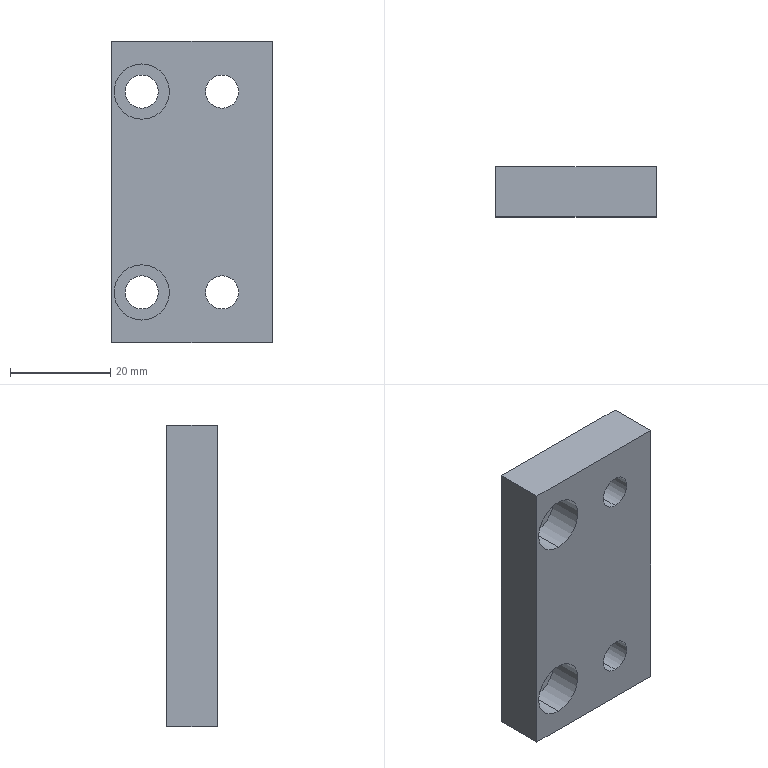Part | STEP file | Tube support mounting bracket base plate | 1 solid | 20 faces | box 32 x 10 x 60 mm | volume 17004 mm3 | cylinder 12 | plane 8 | commonest cylinder face diameters 6.6 x8 11 x4
STEP:
#1=CARTESIAN_POINT('',(0.,0.,0.));
#2=DIRECTION('',(0.,0.,1.));
#3=DIRECTION('',(1.,0.,0.));
#4=AXIS2_PLACEMENT_3D('',#1,#2,#3);
#5=CARTESIAN_POINT('',(6.,0.,23.3));
#6=VERTEX_POINT('',#5);
#7=CARTESIAN_POINT('',(6.,10.,23.3));
#8=VERTEX_POINT('',#7);
#9=CARTESIAN_POINT('',(6.,10.,23.3));
#10=DIRECTION('',(0.,1.,0.));
#11=VECTOR('',#10,1.);
#12=LINE('',#9,#11);
#13=CARTESIAN_POINT('',(6.,10.,20.));
#14=DIRECTION('',(0.,1.,0.));
#15=DIRECTION('',(0.,0.,1.));
#16=AXIS2_PLACEMENT_3D('',#13,#14,#15);
#17=CYLINDRICAL_SURFACE('',#16,3.3);
#18=CARTESIAN_POINT('',(6.283,0.));
#19=DIRECTION('',(0.,1.));
#20=VECTOR('',#19,1.);
#21=LINE('',#18,#20);
#22=(GEOMETRIC_REPRESENTATION_CONTEXT(2)PARAMETRIC_REPRESENTATION_CONTEXT()REPRESENTATION_CONTEXT('',''));
#23=DEFINITIONAL_REPRESENTATION('',(#21),#22);
#24=PCURVE('',#17,#23);
#25=CARTESIAN_POINT('',(6.,10.,20.));
#26=DIRECTION('',(0.,1.,0.));
#27=DIRECTION('',(0.,0.,1.));
#28=AXIS2_PLACEMENT_3D('',#25,#26,#27);
#29=CYLINDRICAL_SURFACE('',#28,3.3);
#30=CARTESIAN_POINT('',(0.,0.));
#31=DIRECTION('',(0.,1.));
#32=VECTOR('',#31,1.);
#33=LINE('',#30,#32);
#34=(GEOMETRIC_REPRESENTATION_CONTEXT(2)PARAMETRIC_REPRESENTATION_CONTEXT()REPRESENTATION_CONTEXT('',''));
#35=DEFINITIONAL_REPRESENTATION('',(#33),#34);
#36=PCURVE('',#29,#35);
#37=SURFACE_CURVE('',#12,(#24,#36),.PCURVE_S1.);
#38=EDGE_CURVE('',#6,#8,#37,.T.);
#39=ORIENTED_EDGE('',*,*,#38,.T.);
#40=CARTESIAN_POINT('',(6.,10.,16.7));
#41=VERTEX_POINT('',#40);
#42=CARTESIAN_POINT('',(6.,10.,20.));
#43=DIRECTION('',(0.,1.,0.));
#44=DIRECTION('',(0.,0.,1.));
#45=AXIS2_PLACEMENT_3D('',#42,#43,#44);
#46=CIRCLE('',#45,3.3);
#47=CARTESIAN_POINT('',(0.,0.));
#48=DIRECTION('',(1.,0.));
#49=VECTOR('',#48,1.);
#50=LINE('',#47,#49);
#51=(GEOMETRIC_REPRESENTATION_CONTEXT(2)PARAMETRIC_REPRESENTATION_CONTEXT()REPRESENTATION_CONTEXT('',''));
#52=DEFINITIONAL_REPRESENTATION('',(#50),#51);
#53=PCURVE('',#17,#52);
#54=CARTESIAN_POINT('',(0.,10.,0.));
#55=DIRECTION('',(0.,-1.,0.));
#56=DIRECTION('',(0.,0.,-1.));
#57=AXIS2_PLACEMENT_3D('',#54,#55,#56);
#58=PLANE('',#57);
#59=CARTESIAN_POINT('',(-23.3,6.));
#60=CARTESIAN_POINT('',(-23.3,11.716));
#61=CARTESIAN_POINT('',(-18.35,8.858));
#62=CARTESIAN_POINT('',(-13.4,6.));
#63=CARTESIAN_POINT('',(-18.35,3.142));
#64=CARTESIAN_POINT('',(-23.3,0.2842));
#65=CARTESIAN_POINT('',(-23.3,6.));
#66=(BOUNDED_CURVE()B_SPLINE_CURVE(2,(#59,#60,#61,#62,#63,#64,#65),.UNSPECIFIED.,.T.,.F.)B_SPLINE_CURVE_WITH_KNOTS((1,2,2,2,2,1),(-2.094,0.,2.094,4.189,6.283,8.378),.UNSPECIFIED.)CURVE()GEOMETRIC_REPRESENTATION_ITEM()RATIONAL_B_SPLINE_CURVE((1.,0.5,1.,0.5,1.,0.5,1.))REPRESENTATION_ITEM(''));
#67=(GEOMETRIC_REPRESENTATION_CONTEXT(2)PARAMETRIC_REPRESENTATION_CONTEXT()REPRESENTATION_CONTEXT('',''));
#68=DEFINITIONAL_REPRESENTATION('',(#66),#67);
#69=PCURVE('',#58,#68);
#70=SURFACE_CURVE('',#46,(#53,#69),.PCURVE_S1.);
#71=EDGE_CURVE('',#41,#8,#70,.T.);
#72=ORIENTED_EDGE('',*,*,#71,.F.);
#73=CARTESIAN_POINT('',(6.,0.,16.7));
#74=VERTEX_POINT('',#73);
#75=CARTESIAN_POINT('',(6.,10.,16.7));
#76=DIRECTION('',(0.,1.,0.));
#77=VECTOR('',#76,1.);
#78=LINE('',#75,#77);
#79=CARTESIAN_POINT('',(3.142,0.));
#80=DIRECTION('',(0.,1.));
#81=VECTOR('',#80,1.);
#82=LINE('',#79,#81);
#83=(GEOMETRIC_REPRESENTATION_CONTEXT(2)PARAMETRIC_REPRESENTATION_CONTEXT()REPRESENTATION_CONTEXT('',''));
#84=DEFINITIONAL_REPRESENTATION('',(#82),#83);
#85=PCURVE('',#17,#84);
#86=CARTESIAN_POINT('',(3.142,0.));
#87=DIRECTION('',(0.,1.));
#88=VECTOR('',#87,1.);
#89=LINE('',#86,#88);
#90=(GEOMETRIC_REPRESENTATION_CONTEXT(2)PARAMETRIC_REPRESENTATION_CONTEXT()REPRESENTATION_CONTEXT('',''));
#91=DEFINITIONAL_REPRESENTATION('',(#89),#90);
#92=PCURVE('',#29,#91);
#93=SURFACE_CURVE('',#78,(#85,#92),.PCURVE_S1.);
#94=EDGE_CURVE('',#74,#41,#93,.T.);
#95=ORIENTED_EDGE('',*,*,#94,.F.);
#96=CARTESIAN_POINT('',(6.,0.,20.));
#97=DIRECTION('',(0.,-1.,0.));
#98=DIRECTION('',(0.,0.,-1.));
#99=AXIS2_PLACEMENT_3D('',#96,#97,#98);
#100=CIRCLE('',#99,3.3);
#101=CARTESIAN_POINT('',(9.425,-10.));
#102=DIRECTION('',(-1.,0.));
#103=VECTOR('',#102,1.);
#104=LINE('',#101,#103);
#105=(GEOMETRIC_REPRESENTATION_CONTEXT(2)PARAMETRIC_REPRESENTATION_CONTEXT()REPRESENTATION_CONTEXT('',''));
#106=DEFINITIONAL_REPRESENTATION('',(#104),#105);
#107=PCURVE('',#17,#106);
#108=CARTESIAN_POINT('',(0.,0.,0.));
#109=DIRECTION('',(0.,-1.,0.));
#110=DIRECTION('',(0.,0.,-1.));
#111=AXIS2_PLACEMENT_3D('',#108,#109,#110);
#112=PLANE('',#111);
#113=CARTESIAN_POINT('',(-20.,6.));
#114=DIRECTION('',(1.,0.));
#115=AXIS2_PLACEMENT_2D('',#113,#114);
#116=CIRCLE('',#115,3.3);
#117=(GEOMETRIC_REPRESENTATION_CONTEXT(2)PARAMETRIC_REPRESENTATION_CONTEXT()REPRESENTATION_CONTEXT('',''));
#118=DEFINITIONAL_REPRESENTATION('',(#116),#117);
#119=PCURVE('',#112,#118);
#120=SURFACE_CURVE('',#100,(#107,#119),.PCURVE_S1.);
#121=EDGE_CURVE('',#6,#74,#120,.T.);
#122=ORIENTED_EDGE('',*,*,#121,.F.);
#123=EDGE_LOOP('',(#39,#72,#95,#122));
#124=FACE_BOUND('',#123,.F.);
#125=ADVANCED_FACE('',(#124),#17,.F.);
#126=CARTESIAN_POINT('',(6.,0.,-16.7));
#127=VERTEX_POINT('',#126);
#128=CARTESIAN_POINT('',(6.,10.,-16.7));
#129=VERTEX_POINT('',#128);
#130=CARTESIAN_POINT('',(6.,10.,-16.7));
#131=DIRECTION('',(0.,1.,0.));
#132=VECTOR('',#131,1.);
#133=LINE('',#130,#132);
#134=CARTESIAN_POINT('',(6.,10.,-20.));
#135=DIRECTION('',(0.,1.,0.));
#136=DIRECTION('',(0.,0.,1.));
#137=AXIS2_PLACEMENT_3D('',#134,#135,#136);
#138=CYLINDRICAL_SURFACE('',#137,3.3);
#139=CARTESIAN_POINT('',(6.283,0.));
#140=DIRECTION('',(0.,1.));
#141=VECTOR('',#140,1.);
#142=LINE('',#139,#141);
#143=(GEOMETRIC_REPRESENTATION_CONTEXT(2)PARAMETRIC_REPRESENTATION_CONTEXT()REPRESENTATION_CONTEXT('',''));
#144=DEFINITIONAL_REPRESENTATION('',(#142),#143);
#145=PCURVE('',#138,#144);
#146=CARTESIAN_POINT('',(6.,10.,-20.));
#147=DIRECTION('',(0.,1.,0.));
#148=DIRECTION('',(0.,0.,1.));
#149=AXIS2_PLACEMENT_3D('',#146,#147,#148);
#150=CYLINDRICAL_SURFACE('',#149,3.3);
#151=CARTESIAN_POINT('',(0.,0.));
#152=DIRECTION('',(0.,1.));
#153=VECTOR('',#152,1.);
#154=LINE('',#151,#153);
#155=(GEOMETRIC_REPRESENTATION_CONTEXT(2)PARAMETRIC_REPRESENTATION_CONTEXT()REPRESENTATION_CONTEXT('',''));
#156=DEFINITIONAL_REPRESENTATION('',(#154),#155);
#157=PCURVE('',#150,#156);
#158=SURFACE_CURVE('',#133,(#145,#157),.PCURVE_S1.);
#159=EDGE_CURVE('',#127,#129,#158,.T.);
#160=ORIENTED_EDGE('',*,*,#159,.T.);
#161=CARTESIAN_POINT('',(6.,10.,-23.3));
#162=VERTEX_POINT('',#161);
#163=CARTESIAN_POINT('',(6.,10.,-20.));
#164=DIRECTION('',(0.,1.,0.));
#165=DIRECTION('',(0.,0.,1.));
#166=AXIS2_PLACEMENT_3D('',#163,#164,#165);
#167=CIRCLE('',#166,3.3);
#168=CARTESIAN_POINT('',(0.,0.));
#169=DIRECTION('',(1.,0.));
#170=VECTOR('',#169,1.);
#171=LINE('',#168,#170);
#172=(GEOMETRIC_REPRESENTATION_CONTEXT(2)PARAMETRIC_REPRESENTATION_CONTEXT()REPRESENTATION_CONTEXT('',''));
#173=DEFINITIONAL_REPRESENTATION('',(#171),#172);
#174=PCURVE('',#138,#173);
#175=CARTESIAN_POINT('',(16.7,6.));
#176=CARTESIAN_POINT('',(16.7,11.716));
#177=CARTESIAN_POINT('',(21.65,8.858));
#178=CARTESIAN_POINT('',(26.6,6.));
#179=CARTESIAN_POINT('',(21.65,3.142));
#180=CARTESIAN_POINT('',(16.7,0.2842));
#181=CARTESIAN_POINT('',(16.7,6.));
#182=(BOUNDED_CURVE()B_SPLINE_CURVE(2,(#175,#176,#177,#178,#179,#180,#181),.UNSPECIFIED.,.T.,.F.)B_SPLINE_CURVE_WITH_KNOTS((1,2,2,2,2,1),(-2.094,0.,2.094,4.189,6.283,8.378),.UNSPECIFIED.)CURVE()GEOMETRIC_REPRESENTATION_ITEM()RATIONAL_B_SPLINE_CURVE((1.,0.5,1.,0.5,1.,0.5,1.))REPRESENTATION_ITEM(''));
#183=(GEOMETRIC_REPRESENTATION_CONTEXT(2)PARAMETRIC_REPRESENTATION_CONTEXT()REPRESENTATION_CONTEXT('',''));
#184=DEFINITIONAL_REPRESENTATION('',(#182),#183);
#185=PCURVE('',#58,#184);
#186=SURFACE_CURVE('',#167,(#174,#185),.PCURVE_S1.);
#187=EDGE_CURVE('',#162,#129,#186,.T.);
#188=ORIENTED_EDGE('',*,*,#187,.F.);
#189=CARTESIAN_POINT('',(6.,0.,-23.3));
#190=VERTEX_POINT('',#189);
#191=CARTESIAN_POINT('',(6.,10.,-23.3));
#192=DIRECTION('',(0.,1.,0.));
#193=VECTOR('',#192,1.);
#194=LINE('',#191,#193);
#195=CARTESIAN_POINT('',(3.142,0.));
#196=DIRECTION('',(0.,1.));
#197=VECTOR('',#196,1.);
#198=LINE('',#195,#197);
#199=(GEOMETRIC_REPRESENTATION_CONTEXT(2)PARAMETRIC_REPRESENTATION_CONTEXT()REPRESENTATION_CONTEXT('',''));
#200=DEFINITIONAL_REPRESENTATION('',(#198),#199);
#201=PCURVE('',#138,#200);
#202=CARTESIAN_POINT('',(3.142,0.));
#203=DIRECTION('',(0.,1.));
#204=VECTOR('',#203,1.);
#205=LINE('',#202,#204);
#206=(GEOMETRIC_REPRESENTATION_CONTEXT(2)PARAMETRIC_REPRESENTATION_CONTEXT()REPRESENTATION_CONTEXT('',''));
#207=DEFINITIONAL_REPRESENTATION('',(#205),#206);
#208=PCURVE('',#150,#207);
#209=SURFACE_CURVE('',#194,(#201,#208),.PCURVE_S1.);
#210=EDGE_CURVE('',#190,#162,#209,.T.);
#211=ORIENTED_EDGE('',*,*,#210,.F.);
#212=CARTESIAN_POINT('',(6.,0.,-20.));
#213=DIRECTION('',(0.,-1.,0.));
#214=DIRECTION('',(0.,0.,-1.));
#215=AXIS2_PLACEMENT_3D('',#212,#213,#214);
#216=CIRCLE('',#215,3.3);
#217=CARTESIAN_POINT('',(9.425,-10.));
#218=DIRECTION('',(-1.,0.));
#219=VECTOR('',#218,1.);
#220=LINE('',#217,#219);
#221=(GEOMETRIC_REPRESENTATION_CONTEXT(2)PARAMETRIC_REPRESENTATION_CONTEXT()REPRESENTATION_CONTEXT('',''));
#222=DEFINITIONAL_REPRESENTATION('',(#220),#221);
#223=PCURVE('',#138,#222);
#224=CARTESIAN_POINT('',(20.,6.));
#225=DIRECTION('',(1.,0.));
#226=AXIS2_PLACEMENT_2D('',#224,#225);
#227=CIRCLE('',#226,3.3);
#228=(GEOMETRIC_REPRESENTATION_CONTEXT(2)PARAMETRIC_REPRESENTATION_CONTEXT()REPRESENTATION_CONTEXT('',''));
#229=DEFINITIONAL_REPRESENTATION('',(#227),#228);
#230=PCURVE('',#112,#229);
#231=SURFACE_CURVE('',#216,(#223,#230),.PCURVE_S1.);
#232=EDGE_CURVE('',#127,#190,#231,.T.);
#233=ORIENTED_EDGE('',*,*,#232,.F.);
#234=EDGE_LOOP('',(#160,#188,#211,#233));
#235=FACE_BOUND('',#234,.F.);
#236=ADVANCED_FACE('',(#235),#138,.F.);
#237=CARTESIAN_POINT('',(-10.,6.8,-25.5));
#238=VERTEX_POINT('',#237);
#239=CARTESIAN_POINT('',(-10.,0.,-25.5));
#240=VERTEX_POINT('',#239);
#241=CARTESIAN_POINT('',(-10.,0.,-25.5));
#242=DIRECTION('',(0.,-1.,0.));
#243=VECTOR('',#242,1.);
#244=LINE('',#241,#243);
#245=CARTESIAN_POINT('',(-10.,0.,-20.));
#246=DIRECTION('',(0.,-1.,0.));
#247=DIRECTION('',(0.,0.,-1.));
#248=AXIS2_PLACEMENT_3D('',#245,#246,#247);
#249=CYLINDRICAL_SURFACE('',#248,5.5);
#250=CARTESIAN_POINT('',(6.283,0.));
#251=DIRECTION('',(0.,1.));
#252=VECTOR('',#251,1.);
#253=LINE('',#250,#252);
#254=(GEOMETRIC_REPRESENTATION_CONTEXT(2)PARAMETRIC_REPRESENTATION_CONTEXT()REPRESENTATION_CONTEXT('',''));
#255=DEFINITIONAL_REPRESENTATION('',(#253),#254);
#256=PCURVE('',#249,#255);
#257=CARTESIAN_POINT('',(-10.,0.,-20.));
#258=DIRECTION('',(0.,-1.,0.));
#259=DIRECTION('',(0.,0.,-1.));
#260=AXIS2_PLACEMENT_3D('',#257,#258,#259);
#261=CYLINDRICAL_SURFACE('',#260,5.5);
#262=CARTESIAN_POINT('',(0.,0.));
#263=DIRECTION('',(0.,1.));
#264=VECTOR('',#263,1.);
#265=LINE('',#262,#264);
#266=(GEOMETRIC_REPRESENTATION_CONTEXT(2)PARAMETRIC_REPRESENTATION_CONTEXT()REPRESENTATION_CONTEXT('',''));
#267=DEFINITIONAL_REPRESENTATION('',(#265),#266);
#268=PCURVE('',#261,#267);
#269=SURFACE_CURVE('',#244,(#256,#268),.PCURVE_S1.);
#270=EDGE_CURVE('',#238,#240,#269,.T.);
#271=ORIENTED_EDGE('',*,*,#270,.T.);
#272=CARTESIAN_POINT('',(-10.,0.,-14.5));
#273=VERTEX_POINT('',#272);
#274=CARTESIAN_POINT('',(-10.,0.,-20.));
#275=DIRECTION('',(0.,-1.,0.));
#276=DIRECTION('',(0.,0.,-1.));
#277=AXIS2_PLACEMENT_3D('',#274,#275,#276);
#278=CIRCLE('',#277,5.5);
#279=CARTESIAN_POINT('',(0.,0.));
#280=DIRECTION('',(1.,0.));
#281=VECTOR('',#280,1.);
#282=LINE('',#279,#281);
#283=(GEOMETRIC_REPRESENTATION_CONTEXT(2)PARAMETRIC_REPRESENTATION_CONTEXT()REPRESENTATION_CONTEXT('',''));
#284=DEFINITIONAL_REPRESENTATION('',(#282),#283);
#285=PCURVE('',#249,#284);
#286=CARTESIAN_POINT('',(20.,-10.));
#287=DIRECTION('',(1.,0.));
#288=AXIS2_PLACEMENT_2D('',#286,#287);
#289=CIRCLE('',#288,5.5);
#290=(GEOMETRIC_REPRESENTATION_CONTEXT(2)PARAMETRIC_REPRESENTATION_CONTEXT()REPRESENTATION_CONTEXT('',''));
#291=DEFINITIONAL_REPRESENTATION('',(#289),#290);
#292=PCURVE('',#112,#291);
#293=SURFACE_CURVE('',#278,(#285,#292),.PCURVE_S1.);
#294=EDGE_CURVE('',#273,#240,#293,.T.);
#295=ORIENTED_EDGE('',*,*,#294,.F.);
#296=CARTESIAN_POINT('',(-10.,6.8,-14.5));
#297=VERTEX_POINT('',#296);
#298=CARTESIAN_POINT('',(-10.,0.,-14.5));
#299=DIRECTION('',(0.,-1.,0.));
#300=VECTOR('',#299,1.);
#301=LINE('',#298,#300);
#302=CARTESIAN_POINT('',(3.142,0.));
#303=DIRECTION('',(0.,1.));
#304=VECTOR('',#303,1.);
#305=LINE('',#302,#304);
#306=(GEOMETRIC_REPRESENTATION_CONTEXT(2)PARAMETRIC_REPRESENTATION_CONTEXT()REPRESENTATION_CONTEXT('',''));
#307=DEFINITIONAL_REPRESENTATION('',(#305),#306);
#308=PCURVE('',#249,#307);
#309=CARTESIAN_POINT('',(3.142,0.));
#310=DIRECTION('',(0.,1.));
#311=VECTOR('',#310,1.);
#312=LINE('',#309,#311);
#313=(GEOMETRIC_REPRESENTATION_CONTEXT(2)PARAMETRIC_REPRESENTATION_CONTEXT()REPRESENTATION_CONTEXT('',''));
#314=DEFINITIONAL_REPRESENTATION('',(#312),#313);
#315=PCURVE('',#261,#314);
#316=SURFACE_CURVE('',#301,(#308,#315),.PCURVE_S1.);
#317=EDGE_CURVE('',#297,#273,#316,.T.);
#318=ORIENTED_EDGE('',*,*,#317,.F.);
#319=CARTESIAN_POINT('',(-10.,6.8,-20.));
#320=DIRECTION('',(0.,-1.,0.));
#321=DIRECTION('',(0.,0.,-1.));
#322=AXIS2_PLACEMENT_3D('',#319,#320,#321);
#323=CIRCLE('',#322,5.5);
#324=CARTESIAN_POINT('',(0.,-6.8));
#325=DIRECTION('',(1.,0.));
#326=VECTOR('',#325,1.);
#327=LINE('',#324,#326);
#328=(GEOMETRIC_REPRESENTATION_CONTEXT(2)PARAMETRIC_REPRESENTATION_CONTEXT()REPRESENTATION_CONTEXT('',''));
#329=DEFINITIONAL_REPRESENTATION('',(#327),#328);
#330=PCURVE('',#249,#329);
#331=CARTESIAN_POINT('',(-6.7,6.8,-20.));
#332=DIRECTION('',(0.,1.,0.));
#333=DIRECTION('',(0.,0.,1.));
#334=AXIS2_PLACEMENT_3D('',#331,#332,#333);
#335=PLANE('',#334);
#336=CARTESIAN_POINT('',(-5.5,-3.3));
#337=CARTESIAN_POINT('',(-5.5,6.226));
#338=CARTESIAN_POINT('',(2.75,1.463));
#339=CARTESIAN_POINT('',(11.,-3.3));
#340=CARTESIAN_POINT('',(2.75,-8.063));
#341=CARTESIAN_POINT('',(-5.5,-12.826));
#342=CARTESIAN_POINT('',(-5.5,-3.3));
#343=(BOUNDED_CURVE()B_SPLINE_CURVE(2,(#336,#337,#338,#339,#340,#341,#342),.UNSPECIFIED.,.T.,.F.)B_SPLINE_CURVE_WITH_KNOTS((1,2,2,2,2,1),(-2.094,0.,2.094,4.189,6.283,8.378),.UNSPECIFIED.)CURVE()GEOMETRIC_REPRESENTATION_ITEM()RATIONAL_B_SPLINE_CURVE((1.,0.5,1.,0.5,1.,0.5,1.))REPRESENTATION_ITEM(''));
#344=(GEOMETRIC_REPRESENTATION_CONTEXT(2)PARAMETRIC_REPRESENTATION_CONTEXT()REPRESENTATION_CONTEXT('',''));
#345=DEFINITIONAL_REPRESENTATION('',(#343),#344);
#346=PCURVE('',#335,#345);
#347=SURFACE_CURVE('',#323,(#330,#346),.PCURVE_S1.);
#348=EDGE_CURVE('',#297,#238,#347,.T.);
#349=ORIENTED_EDGE('',*,*,#348,.T.);
#350=EDGE_LOOP('',(#271,#295,#318,#349));
#351=FACE_BOUND('',#350,.F.);
#352=ADVANCED_FACE('',(#351),#249,.F.);
#353=CARTESIAN_POINT('',(-10.,10.,-23.3));
#354=VERTEX_POINT('',#353);
#355=CARTESIAN_POINT('',(-10.,6.8,-23.3));
#356=VERTEX_POINT('',#355);
#357=CARTESIAN_POINT('',(-10.,0.,-23.3));
#358=DIRECTION('',(0.,-1.,0.));
#359=VECTOR('',#358,1.);
#360=LINE('',#357,#359);
#361=CARTESIAN_POINT('',(-10.,0.,-20.));
#362=DIRECTION('',(0.,-1.,0.));
#363=DIRECTION('',(0.,0.,-1.));
#364=AXIS2_PLACEMENT_3D('',#361,#362,#363);
#365=CYLINDRICAL_SURFACE('',#364,3.3);
#366=CARTESIAN_POINT('',(6.283,0.));
#367=DIRECTION('',(0.,1.));
#368=VECTOR('',#367,1.);
#369=LINE('',#366,#368);
#370=(GEOMETRIC_REPRESENTATION_CONTEXT(2)PARAMETRIC_REPRESENTATION_CONTEXT()REPRESENTATION_CONTEXT('',''));
#371=DEFINITIONAL_REPRESENTATION('',(#369),#370);
#372=PCURVE('',#365,#371);
#373=CARTESIAN_POINT('',(-10.,0.,-20.));
#374=DIRECTION('',(0.,-1.,0.));
#375=DIRECTION('',(0.,0.,-1.));
#376=AXIS2_PLACEMENT_3D('',#373,#374,#375);
#377=CYLINDRICAL_SURFACE('',#376,3.3);
#378=CARTESIAN_POINT('',(0.,0.));
#379=DIRECTION('',(0.,1.));
#380=VECTOR('',#379,1.);
#381=LINE('',#378,#380);
#382=(GEOMETRIC_REPRESENTATION_CONTEXT(2)PARAMETRIC_REPRESENTATION_CONTEXT()REPRESENTATION_CONTEXT('',''));
#383=DEFINITIONAL_REPRESENTATION('',(#381),#382);
#384=PCURVE('',#377,#383);
#385=SURFACE_CURVE('',#360,(#372,#384),.PCURVE_S1.);
#386=EDGE_CURVE('',#354,#356,#385,.T.);
#387=ORIENTED_EDGE('',*,*,#386,.T.);
#388=CARTESIAN_POINT('',(-10.,6.8,-16.7));
#389=VERTEX_POINT('',#388);
#390=CARTESIAN_POINT('',(-10.,6.8,-20.));
#391=DIRECTION('',(0.,-1.,0.));
#392=DIRECTION('',(0.,0.,-1.));
#393=AXIS2_PLACEMENT_3D('',#390,#391,#392);
#394=CIRCLE('',#393,3.3);
#395=CARTESIAN_POINT('',(0.,-6.8));
#396=DIRECTION('',(1.,0.));
#397=VECTOR('',#396,1.);
#398=LINE('',#395,#397);
#399=(GEOMETRIC_REPRESENTATION_CONTEXT(2)PARAMETRIC_REPRESENTATION_CONTEXT()REPRESENTATION_CONTEXT('',''));
#400=DEFINITIONAL_REPRESENTATION('',(#398),#399);
#401=PCURVE('',#365,#400);
#402=CARTESIAN_POINT('',(-3.3,-3.3));
#403=CARTESIAN_POINT('',(-3.3,2.416));
#404=CARTESIAN_POINT('',(1.65,-0.4421));
#405=CARTESIAN_POINT('',(6.6,-3.3));
#406=CARTESIAN_POINT('',(1.65,-6.158));
#407=CARTESIAN_POINT('',(-3.3,-9.016));
#408=CARTESIAN_POINT('',(-3.3,-3.3));
#409=(BOUNDED_CURVE()B_SPLINE_CURVE(2,(#402,#403,#404,#405,#406,#407,#408),.UNSPECIFIED.,.T.,.F.)B_SPLINE_CURVE_WITH_KNOTS((1,2,2,2,2,1),(-2.094,0.,2.094,4.189,6.283,8.378),.UNSPECIFIED.)CURVE()GEOMETRIC_REPRESENTATION_ITEM()RATIONAL_B_SPLINE_CURVE((1.,0.5,1.,0.5,1.,0.5,1.))REPRESENTATION_ITEM(''));
#410=(GEOMETRIC_REPRESENTATION_CONTEXT(2)PARAMETRIC_REPRESENTATION_CONTEXT()REPRESENTATION_CONTEXT('',''));
#411=DEFINITIONAL_REPRESENTATION('',(#409),#410);
#412=PCURVE('',#335,#411);
#413=SURFACE_CURVE('',#394,(#401,#412),.PCURVE_S1.);
#414=EDGE_CURVE('',#389,#356,#413,.T.);
#415=ORIENTED_EDGE('',*,*,#414,.F.);
#416=CARTESIAN_POINT('',(-10.,10.,-16.7));
#417=VERTEX_POINT('',#416);
#418=CARTESIAN_POINT('',(-10.,0.,-16.7));
#419=DIRECTION('',(0.,-1.,0.));
#420=VECTOR('',#419,1.);
#421=LINE('',#418,#420);
#422=CARTESIAN_POINT('',(3.142,0.));
#423=DIRECTION('',(0.,1.));
#424=VECTOR('',#423,1.);
#425=LINE('',#422,#424);
#426=(GEOMETRIC_REPRESENTATION_CONTEXT(2)PARAMETRIC_REPRESENTATION_CONTEXT()REPRESENTATION_CONTEXT('',''));
#427=DEFINITIONAL_REPRESENTATION('',(#425),#426);
#428=PCURVE('',#365,#427);
#429=CARTESIAN_POINT('',(3.142,0.));
#430=DIRECTION('',(0.,1.));
#431=VECTOR('',#430,1.);
#432=LINE('',#429,#431);
#433=(GEOMETRIC_REPRESENTATION_CONTEXT(2)PARAMETRIC_REPRESENTATION_CONTEXT()REPRESENTATION_CONTEXT('',''));
#434=DEFINITIONAL_REPRESENTATION('',(#432),#433);
#435=PCURVE('',#377,#434);
#436=SURFACE_CURVE('',#421,(#428,#435),.PCURVE_S1.);
#437=EDGE_CURVE('',#417,#389,#436,.T.);
#438=ORIENTED_EDGE('',*,*,#437,.F.);
#439=CARTESIAN_POINT('',(-10.,10.,-20.));
#440=DIRECTION('',(0.,-1.,0.));
#441=DIRECTION('',(0.,0.,-1.));
#442=AXIS2_PLACEMENT_3D('',#439,#440,#441);
#443=CIRCLE('',#442,3.3);
#444=CARTESIAN_POINT('',(0.,-10.));
#445=DIRECTION('',(1.,0.));
#446=VECTOR('',#445,1.);
#447=LINE('',#444,#446);
#448=(GEOMETRIC_REPRESENTATION_CONTEXT(2)PARAMETRIC_REPRESENTATION_CONTEXT()REPRESENTATION_CONTEXT('',''));
#449=DEFINITIONAL_REPRESENTATION('',(#447),#448);
#450=PCURVE('',#365,#449);
#451=CARTESIAN_POINT('',(20.,-10.));
#452=DIRECTION('',(1.,0.));
#453=AXIS2_PLACEMENT_2D('',#451,#452);
#454=CIRCLE('',#453,3.3);
#455=(GEOMETRIC_REPRESENTATION_CONTEXT(2)PARAMETRIC_REPRESENTATION_CONTEXT()REPRESENTATION_CONTEXT('',''));
#456=DEFINITIONAL_REPRESENTATION('',(#454),#455);
#457=PCURVE('',#58,#456);
#458=SURFACE_CURVE('',#443,(#450,#457),.PCURVE_S1.);
#459=EDGE_CURVE('',#417,#354,#458,.T.);
#460=ORIENTED_EDGE('',*,*,#459,.T.);
#461=EDGE_LOOP('',(#387,#415,#438,#460));
#462=FACE_BOUND('',#461,.F.);
#463=ADVANCED_FACE('',(#462),#365,.F.);
#464=CARTESIAN_POINT('',(-10.,6.8,14.5));
#465=VERTEX_POINT('',#464);
#466=CARTESIAN_POINT('',(-10.,0.,14.5));
#467=VERTEX_POINT('',#466);
#468=CARTESIAN_POINT('',(-10.,0.,14.5));
#469=DIRECTION('',(0.,-1.,0.));
#470=VECTOR('',#469,1.);
#471=LINE('',#468,#470);
#472=CARTESIAN_POINT('',(-10.,0.,20.));
#473=DIRECTION('',(0.,-1.,0.));
#474=DIRECTION('',(0.,0.,-1.));
#475=AXIS2_PLACEMENT_3D('',#472,#473,#474);
#476=CYLINDRICAL_SURFACE('',#475,5.5);
#477=CARTESIAN_POINT('',(6.283,0.));
#478=DIRECTION('',(0.,1.));
#479=VECTOR('',#478,1.);
#480=LINE('',#477,#479);
#481=(GEOMETRIC_REPRESENTATION_CONTEXT(2)PARAMETRIC_REPRESENTATION_CONTEXT()REPRESENTATION_CONTEXT('',''));
#482=DEFINITIONAL_REPRESENTATION('',(#480),#481);
#483=PCURVE('',#476,#482);
#484=CARTESIAN_POINT('',(-10.,0.,20.));
#485=DIRECTION('',(0.,-1.,0.));
#486=DIRECTION('',(0.,0.,-1.));
#487=AXIS2_PLACEMENT_3D('',#484,#485,#486);
#488=CYLINDRICAL_SURFACE('',#487,5.5);
#489=CARTESIAN_POINT('',(0.,0.));
#490=DIRECTION('',(0.,1.));
#491=VECTOR('',#490,1.);
#492=LINE('',#489,#491);
#493=(GEOMETRIC_REPRESENTATION_CONTEXT(2)PARAMETRIC_REPRESENTATION_CONTEXT()REPRESENTATION_CONTEXT('',''));
#494=DEFINITIONAL_REPRESENTATION('',(#492),#493);
#495=PCURVE('',#488,#494);
#496=SURFACE_CURVE('',#471,(#483,#495),.PCURVE_S1.);
#497=EDGE_CURVE('',#465,#467,#496,.T.);
#498=ORIENTED_EDGE('',*,*,#497,.T.);
#499=CARTESIAN_POINT('',(-10.,0.,25.5));
#500=VERTEX_POINT('',#499);
#501=CARTESIAN_POINT('',(-10.,0.,20.));
#502=DIRECTION('',(0.,-1.,0.));
#503=DIRECTION('',(0.,0.,-1.));
#504=AXIS2_PLACEMENT_3D('',#501,#502,#503);
#505=CIRCLE('',#504,5.5);
#506=CARTESIAN_POINT('',(0.,0.));
#507=DIRECTION('',(1.,0.));
#508=VECTOR('',#507,1.);
#509=LINE('',#506,#508);
#510=(GEOMETRIC_REPRESENTATION_CONTEXT(2)PARAMETRIC_REPRESENTATION_CONTEXT()REPRESENTATION_CONTEXT('',''));
#511=DEFINITIONAL_REPRESENTATION('',(#509),#510);
#512=PCURVE('',#476,#511);
#513=CARTESIAN_POINT('',(-20.,-10.));
#514=DIRECTION('',(1.,0.));
#515=AXIS2_PLACEMENT_2D('',#513,#514);
#516=CIRCLE('',#515,5.5);
#517=(GEOMETRIC_REPRESENTATION_CONTEXT(2)PARAMETRIC_REPRESENTATION_CONTEXT()REPRESENTATION_CONTEXT('',''));
#518=DEFINITIONAL_REPRESENTATION('',(#516),#517);
#519=PCURVE('',#112,#518);
#520=SURFACE_CURVE('',#505,(#512,#519),.PCURVE_S1.);
#521=EDGE_CURVE('',#500,#467,#520,.T.);
#522=ORIENTED_EDGE('',*,*,#521,.F.);
#523=CARTESIAN_POINT('',(-10.,6.8,25.5));
#524=VERTEX_POINT('',#523);
#525=CARTESIAN_POINT('',(-10.,0.,25.5));
#526=DIRECTION('',(0.,-1.,0.));
#527=VECTOR('',#526,1.);
#528=LINE('',#525,#527);
#529=CARTESIAN_POINT('',(3.142,0.));
#530=DIRECTION('',(0.,1.));
#531=VECTOR('',#530,1.);
#532=LINE('',#529,#531);
#533=(GEOMETRIC_REPRESENTATION_CONTEXT(2)PARAMETRIC_REPRESENTATION_CONTEXT()REPRESENTATION_CONTEXT('',''));
#534=DEFINITIONAL_REPRESENTATION('',(#532),#533);
#535=PCURVE('',#476,#534);
#536=CARTESIAN_POINT('',(3.142,0.));
#537=DIRECTION('',(0.,1.));
#538=VECTOR('',#537,1.);
#539=LINE('',#536,#538);
#540=(GEOMETRIC_REPRESENTATION_CONTEXT(2)PARAMETRIC_REPRESENTATION_CONTEXT()REPRESENTATION_CONTEXT('',''));
#541=DEFINITIONAL_REPRESENTATION('',(#539),#540);
#542=PCURVE('',#488,#541);
#543=SURFACE_CURVE('',#528,(#535,#542),.PCURVE_S1.);
#544=EDGE_CURVE('',#524,#500,#543,.T.);
#545=ORIENTED_EDGE('',*,*,#544,.F.);
#546=CARTESIAN_POINT('',(-10.,6.8,20.));
#547=DIRECTION('',(0.,-1.,0.));
#548=DIRECTION('',(0.,0.,-1.));
#549=AXIS2_PLACEMENT_3D('',#546,#547,#548);
#550=CIRCLE('',#549,5.5);
#551=CARTESIAN_POINT('',(0.,-6.8));
#552=DIRECTION('',(1.,0.));
#553=VECTOR('',#552,1.);
#554=LINE('',#551,#553);
#555=(GEOMETRIC_REPRESENTATION_CONTEXT(2)PARAMETRIC_REPRESENTATION_CONTEXT()REPRESENTATION_CONTEXT('',''));
#556=DEFINITIONAL_REPRESENTATION('',(#554),#555);
#557=PCURVE('',#476,#556);
#558=CARTESIAN_POINT('',(-6.7,6.8,20.));
#559=DIRECTION('',(0.,1.,0.));
#560=DIRECTION('',(0.,0.,1.));
#561=AXIS2_PLACEMENT_3D('',#558,#559,#560);
#562=PLANE('',#561);
#563=CARTESIAN_POINT('',(-5.5,-3.3));
#564=CARTESIAN_POINT('',(-5.5,6.226));
#565=CARTESIAN_POINT('',(2.75,1.463));
#566=CARTESIAN_POINT('',(11.,-3.3));
#567=CARTESIAN_POINT('',(2.75,-8.063));
#568=CARTESIAN_POINT('',(-5.5,-12.826));
#569=CARTESIAN_POINT('',(-5.5,-3.3));
#570=(BOUNDED_CURVE()B_SPLINE_CURVE(2,(#563,#564,#565,#566,#567,#568,#569),.UNSPECIFIED.,.T.,.F.)B_SPLINE_CURVE_WITH_KNOTS((1,2,2,2,2,1),(-2.094,0.,2.094,4.189,6.283,8.378),.UNSPECIFIED.)CURVE()GEOMETRIC_REPRESENTATION_ITEM()RATIONAL_B_SPLINE_CURVE((1.,0.5,1.,0.5,1.,0.5,1.))REPRESENTATION_ITEM(''));
#571=(GEOMETRIC_REPRESENTATION_CONTEXT(2)PARAMETRIC_REPRESENTATION_CONTEXT()REPRESENTATION_CONTEXT('',''));
#572=DEFINITIONAL_REPRESENTATION('',(#570),#571);
#573=PCURVE('',#562,#572);
#574=SURFACE_CURVE('',#550,(#557,#573),.PCURVE_S1.);
#575=EDGE_CURVE('',#524,#465,#574,.T.);
#576=ORIENTED_EDGE('',*,*,#575,.T.);
#577=EDGE_LOOP('',(#498,#522,#545,#576));
#578=FACE_BOUND('',#577,.F.);
#579=ADVANCED_FACE('',(#578),#476,.F.);
#580=CARTESIAN_POINT('',(-10.,10.,16.7));
#581=VERTEX_POINT('',#580);
#582=CARTESIAN_POINT('',(-10.,6.8,16.7));
#583=VERTEX_POINT('',#582);
#584=CARTESIAN_POINT('',(-10.,0.,16.7));
#585=DIRECTION('',(0.,-1.,0.));
#586=VECTOR('',#585,1.);
#587=LINE('',#584,#586);
#588=CARTESIAN_POINT('',(-10.,0.,20.));
#589=DIRECTION('',(0.,-1.,0.));
#590=DIRECTION('',(0.,0.,-1.));
#591=AXIS2_PLACEMENT_3D('',#588,#589,#590);
#592=CYLINDRICAL_SURFACE('',#591,3.3);
#593=CARTESIAN_POINT('',(6.283,0.));
#594=DIRECTION('',(0.,1.));
#595=VECTOR('',#594,1.);
#596=LINE('',#593,#595);
#597=(GEOMETRIC_REPRESENTATION_CONTEXT(2)PARAMETRIC_REPRESENTATION_CONTEXT()REPRESENTATION_CONTEXT('',''));
#598=DEFINITIONAL_REPRESENTATION('',(#596),#597);
#599=PCURVE('',#592,#598);
#600=CARTESIAN_POINT('',(-10.,0.,20.));
#601=DIRECTION('',(0.,-1.,0.));
#602=DIRECTION('',(0.,0.,-1.));
#603=AXIS2_PLACEMENT_3D('',#600,#601,#602);
#604=CYLINDRICAL_SURFACE('',#603,3.3);
#605=CARTESIAN_POINT('',(0.,0.));
#606=DIRECTION('',(0.,1.));
#607=VECTOR('',#606,1.);
#608=LINE('',#605,#607);
#609=(GEOMETRIC_REPRESENTATION_CONTEXT(2)PARAMETRIC_REPRESENTATION_CONTEXT()REPRESENTATION_CONTEXT('',''));
#610=DEFINITIONAL_REPRESENTATION('',(#608),#609);
#611=PCURVE('',#604,#610);
#612=SURFACE_CURVE('',#587,(#599,#611),.PCURVE_S1.);
#613=EDGE_CURVE('',#581,#583,#612,.T.);
#614=ORIENTED_EDGE('',*,*,#613,.T.);
#615=CARTESIAN_POINT('',(-10.,6.8,23.3));
#616=VERTEX_POINT('',#615);
#617=CARTESIAN_POINT('',(-10.,6.8,20.));
#618=DIRECTION('',(0.,-1.,0.));
#619=DIRECTION('',(0.,0.,-1.));
#620=AXIS2_PLACEMENT_3D('',#617,#618,#619);
#621=CIRCLE('',#620,3.3);
#622=CARTESIAN_POINT('',(0.,-6.8));
#623=DIRECTION('',(1.,0.));
#624=VECTOR('',#623,1.);
#625=LINE('',#622,#624);
#626=(GEOMETRIC_REPRESENTATION_CONTEXT(2)PARAMETRIC_REPRESENTATION_CONTEXT()REPRESENTATION_CONTEXT('',''));
#627=DEFINITIONAL_REPRESENTATION('',(#625),#626);
#628=PCURVE('',#592,#627);
#629=CARTESIAN_POINT('',(-3.3,-3.3));
#630=CARTESIAN_POINT('',(-3.3,2.416));
#631=CARTESIAN_POINT('',(1.65,-0.4421));
#632=CARTESIAN_POINT('',(6.6,-3.3));
#633=CARTESIAN_POINT('',(1.65,-6.158));
#634=CARTESIAN_POINT('',(-3.3,-9.016));
#635=CARTESIAN_POINT('',(-3.3,-3.3));
#636=(BOUNDED_CURVE()B_SPLINE_CURVE(2,(#629,#630,#631,#632,#633,#634,#635),.UNSPECIFIED.,.T.,.F.)B_SPLINE_CURVE_WITH_KNOTS((1,2,2,2,2,1),(-2.094,0.,2.094,4.189,6.283,8.378),.UNSPECIFIED.)CURVE()GEOMETRIC_REPRESENTATION_ITEM()RATIONAL_B_SPLINE_CURVE((1.,0.5,1.,0.5,1.,0.5,1.))REPRESENTATION_ITEM(''));
#637=(GEOMETRIC_REPRESENTATION_CONTEXT(2)PARAMETRIC_REPRESENTATION_CONTEXT()REPRESENTATION_CONTEXT('',''));
#638=DEFINITIONAL_REPRESENTATION('',(#636),#637);
#639=PCURVE('',#562,#638);
#640=SURFACE_CURVE('',#621,(#628,#639),.PCURVE_S1.);
#641=EDGE_CURVE('',#616,#583,#640,.T.);
#642=ORIENTED_EDGE('',*,*,#641,.F.);
#643=CARTESIAN_POINT('',(-10.,10.,23.3));
#644=VERTEX_POINT('',#643);
#645=CARTESIAN_POINT('',(-10.,0.,23.3));
#646=DIRECTION('',(0.,-1.,0.));
#647=VECTOR('',#646,1.);
#648=LINE('',#645,#647);
#649=CARTESIAN_POINT('',(3.142,0.));
#650=DIRECTION('',(0.,1.));
#651=VECTOR('',#650,1.);
#652=LINE('',#649,#651);
#653=(GEOMETRIC_REPRESENTATION_CONTEXT(2)PARAMETRIC_REPRESENTATION_CONTEXT()REPRESENTATION_CONTEXT('',''));
#654=DEFINITIONAL_REPRESENTATION('',(#652),#653);
#655=PCURVE('',#592,#654);
#656=CARTESIAN_POINT('',(3.142,0.));
#657=DIRECTION('',(0.,1.));
#658=VECTOR('',#657,1.);
#659=LINE('',#656,#658);
#660=(GEOMETRIC_REPRESENTATION_CONTEXT(2)PARAMETRIC_REPRESENTATION_CONTEXT()REPRESENTATION_CONTEXT('',''));
#661=DEFINITIONAL_REPRESENTATION('',(#659),#660);
#662=PCURVE('',#604,#661);
#663=SURFACE_CURVE('',#648,(#655,#662),.PCURVE_S1.);
#664=EDGE_CURVE('',#644,#616,#663,.T.);
#665=ORIENTED_EDGE('',*,*,#664,.F.);
#666=CARTESIAN_POINT('',(-10.,10.,20.));
#667=DIRECTION('',(0.,-1.,0.));
#668=DIRECTION('',(0.,0.,-1.));
#669=AXIS2_PLACEMENT_3D('',#666,#667,#668);
#670=CIRCLE('',#669,3.3);
#671=CARTESIAN_POINT('',(0.,-10.));
#672=DIRECTION('',(1.,0.));
#673=VECTOR('',#672,1.);
#674=LINE('',#671,#673);
#675=(GEOMETRIC_REPRESENTATION_CONTEXT(2)PARAMETRIC_REPRESENTATION_CONTEXT()REPRESENTATION_CONTEXT('',''));
#676=DEFINITIONAL_REPRESENTATION('',(#674),#675);
#677=PCURVE('',#592,#676);
#678=CARTESIAN_POINT('',(-20.,-10.));
#679=DIRECTION('',(1.,0.));
#680=AXIS2_PLACEMENT_2D('',#678,#679);
#681=CIRCLE('',#680,3.3);
#682=(GEOMETRIC_REPRESENTATION_CONTEXT(2)PARAMETRIC_REPRESENTATION_CONTEXT()REPRESENTATION_CONTEXT('',''));
#683=DEFINITIONAL_REPRESENTATION('',(#681),#682);
#684=PCURVE('',#58,#683);
#685=SURFACE_CURVE('',#670,(#677,#684),.PCURVE_S1.);
#686=EDGE_CURVE('',#644,#581,#685,.T.);
#687=ORIENTED_EDGE('',*,*,#686,.T.);
#688=EDGE_LOOP('',(#614,#642,#665,#687));
#689=FACE_BOUND('',#688,.F.);
#690=ADVANCED_FACE('',(#689),#592,.F.);
#691=CARTESIAN_POINT('',(16.,0.,30.));
#692=VERTEX_POINT('',#691);
#693=CARTESIAN_POINT('',(16.,0.,-30.));
#694=VERTEX_POINT('',#693);
#695=CARTESIAN_POINT('',(16.,0.,30.));
#696=DIRECTION('',(0.,0.,-1.));
#697=VECTOR('',#696,1.);
#698=LINE('',#695,#697);
#699=CARTESIAN_POINT('',(16.,10.,30.));
#700=DIRECTION('',(-1.,0.,0.));
#701=DIRECTION('',(0.,0.,1.));
#702=AXIS2_PLACEMENT_3D('',#699,#700,#701);
#703=PLANE('',#702);
#704=CARTESIAN_POINT('',(0.,-10.));
#705=DIRECTION('',(-1.,0.));
#706=VECTOR('',#705,1.);
#707=LINE('',#704,#706);
#708=(GEOMETRIC_REPRESENTATION_CONTEXT(2)PARAMETRIC_REPRESENTATION_CONTEXT()REPRESENTATION_CONTEXT('',''));
#709=DEFINITIONAL_REPRESENTATION('',(#707),#708);
#710=PCURVE('',#703,#709);
#711=CARTESIAN_POINT('',(-30.,16.));
#712=DIRECTION('',(1.,0.));
#713=VECTOR('',#712,1.);
#714=LINE('',#711,#713);
#715=(GEOMETRIC_REPRESENTATION_CONTEXT(2)PARAMETRIC_REPRESENTATION_CONTEXT()REPRESENTATION_CONTEXT('',''));
#716=DEFINITIONAL_REPRESENTATION('',(#714),#715);
#717=PCURVE('',#112,#716);
#718=SURFACE_CURVE('',#698,(#710,#717),.PCURVE_S1.);
#719=EDGE_CURVE('',#692,#694,#718,.T.);
#720=ORIENTED_EDGE('',*,*,#719,.T.);
#721=CARTESIAN_POINT('',(16.,10.,-30.));
#722=VERTEX_POINT('',#721);
#723=CARTESIAN_POINT('',(16.,10.,-30.));
#724=DIRECTION('',(0.,-1.,0.));
#725=VECTOR('',#724,1.);
#726=LINE('',#723,#725);
#727=CARTESIAN_POINT('',(-60.,0.));
#728=DIRECTION('',(0.,-1.));
#729=VECTOR('',#728,1.);
#730=LINE('',#727,#729);
#731=(GEOMETRIC_REPRESENTATION_CONTEXT(2)PARAMETRIC_REPRESENTATION_CONTEXT()REPRESENTATION_CONTEXT('',''));
#732=DEFINITIONAL_REPRESENTATION('',(#730),#731);
#733=PCURVE('',#703,#732);
#734=CARTESIAN_POINT('',(-16.,10.,-30.));
#735=DIRECTION('',(0.,0.,1.));
#736=DIRECTION('',(1.,0.,0.));
#737=AXIS2_PLACEMENT_3D('',#734,#735,#736);
#738=PLANE('',#737);
#739=CARTESIAN_POINT('',(32.,0.));
#740=DIRECTION('',(0.,-1.));
#741=VECTOR('',#740,1.);
#742=LINE('',#739,#741);
#743=(GEOMETRIC_REPRESENTATION_CONTEXT(2)PARAMETRIC_REPRESENTATION_CONTEXT()REPRESENTATION_CONTEXT('',''));
#744=DEFINITIONAL_REPRESENTATION('',(#742),#743);
#745=PCURVE('',#738,#744);
#746=SURFACE_CURVE('',#726,(#733,#745),.PCURVE_S1.);
#747=EDGE_CURVE('',#722,#694,#746,.T.);
#748=ORIENTED_EDGE('',*,*,#747,.F.);
#749=CARTESIAN_POINT('',(16.,10.,30.));
#750=VERTEX_POINT('',#749);
#751=CARTESIAN_POINT('',(16.,10.,30.));
#752=DIRECTION('',(0.,0.,-1.));
#753=VECTOR('',#752,1.);
#754=LINE('',#751,#753);
#755=CARTESIAN_POINT('',(0.,0.));
#756=DIRECTION('',(-1.,0.));
#757=VECTOR('',#756,1.);
#758=LINE('',#755,#757);
#759=(GEOMETRIC_REPRESENTATION_CONTEXT(2)PARAMETRIC_REPRESENTATION_CONTEXT()REPRESENTATION_CONTEXT('',''));
#760=DEFINITIONAL_REPRESENTATION('',(#758),#759);
#761=PCURVE('',#703,#760);
#762=CARTESIAN_POINT('',(-30.,16.));
#763=DIRECTION('',(1.,0.));
#764=VECTOR('',#763,1.);
#765=LINE('',#762,#764);
#766=(GEOMETRIC_REPRESENTATION_CONTEXT(2)PARAMETRIC_REPRESENTATION_CONTEXT()REPRESENTATION_CONTEXT('',''));
#767=DEFINITIONAL_REPRESENTATION('',(#765),#766);
#768=PCURVE('',#58,#767);
#769=SURFACE_CURVE('',#754,(#761,#768),.PCURVE_S1.);
#770=EDGE_CURVE('',#750,#722,#769,.T.);
#771=ORIENTED_EDGE('',*,*,#770,.F.);
#772=CARTESIAN_POINT('',(16.,10.,30.));
#773=DIRECTION('',(0.,-1.,0.));
#774=VECTOR('',#773,1.);
#775=LINE('',#772,#774);
#776=CARTESIAN_POINT('',(0.,0.));
#777=DIRECTION('',(0.,-1.));
#778=VECTOR('',#777,1.);
#779=LINE('',#776,#778);
#780=(GEOMETRIC_REPRESENTATION_CONTEXT(2)PARAMETRIC_REPRESENTATION_CONTEXT()REPRESENTATION_CONTEXT('',''));
#781=DEFINITIONAL_REPRESENTATION('',(#779),#780);
#782=PCURVE('',#703,#781);
#783=CARTESIAN_POINT('',(-16.,10.,30.));
#784=DIRECTION('',(0.,0.,-1.));
#785=DIRECTION('',(-1.,0.,0.));
#786=AXIS2_PLACEMENT_3D('',#783,#784,#785);
#787=PLANE('',#786);
#788=CARTESIAN_POINT('',(-32.,0.));
#789=DIRECTION('',(0.,-1.));
#790=VECTOR('',#789,1.);
#791=LINE('',#788,#790);
#792=(GEOMETRIC_REPRESENTATION_CONTEXT(2)PARAMETRIC_REPRESENTATION_CONTEXT()REPRESENTATION_CONTEXT('',''));
#793=DEFINITIONAL_REPRESENTATION('',(#791),#792);
#794=PCURVE('',#787,#793);
#795=SURFACE_CURVE('',#775,(#782,#794),.PCURVE_S1.);
#796=EDGE_CURVE('',#750,#692,#795,.T.);
#797=ORIENTED_EDGE('',*,*,#796,.T.);
#798=EDGE_LOOP('',(#720,#748,#771,#797));
#799=FACE_BOUND('',#798,.T.);
#800=ADVANCED_FACE('',(#799),#703,.F.);
#801=CARTESIAN_POINT('',(-16.,0.,-30.));
#802=VERTEX_POINT('',#801);
#803=CARTESIAN_POINT('',(-16.,0.,-30.));
#804=DIRECTION('',(-1.,0.,0.));
#805=VECTOR('',#804,1.);
#806=LINE('',#803,#805);
#807=CARTESIAN_POINT('',(0.,-10.));
#808=DIRECTION('',(-1.,0.));
#809=VECTOR('',#808,1.);
#810=LINE('',#807,#809);
#811=(GEOMETRIC_REPRESENTATION_CONTEXT(2)PARAMETRIC_REPRESENTATION_CONTEXT()REPRESENTATION_CONTEXT('',''));
#812=DEFINITIONAL_REPRESENTATION('',(#810),#811);
#813=PCURVE('',#738,#812);
#814=CARTESIAN_POINT('',(30.,-16.));
#815=DIRECTION('',(0.,-1.));
#816=VECTOR('',#815,1.);
#817=LINE('',#814,#816);
#818=(GEOMETRIC_REPRESENTATION_CONTEXT(2)PARAMETRIC_REPRESENTATION_CONTEXT()REPRESENTATION_CONTEXT('',''));
#819=DEFINITIONAL_REPRESENTATION('',(#817),#818);
#820=PCURVE('',#112,#819);
#821=SURFACE_CURVE('',#806,(#813,#820),.PCURVE_S1.);
#822=EDGE_CURVE('',#694,#802,#821,.T.);
#823=ORIENTED_EDGE('',*,*,#822,.T.);
#824=CARTESIAN_POINT('',(-16.,10.,-30.));
#825=VERTEX_POINT('',#824);
#826=CARTESIAN_POINT('',(-16.,10.,-30.));
#827=DIRECTION('',(0.,-1.,0.));
#828=VECTOR('',#827,1.);
#829=LINE('',#826,#828);
#830=CARTESIAN_POINT('',(0.,0.));
#831=DIRECTION('',(0.,-1.));
#832=VECTOR('',#831,1.);
#833=LINE('',#830,#832);
#834=(GEOMETRIC_REPRESENTATION_CONTEXT(2)PARAMETRIC_REPRESENTATION_CONTEXT()REPRESENTATION_CONTEXT('',''));
#835=DEFINITIONAL_REPRESENTATION('',(#833),#834);
#836=PCURVE('',#738,#835);
#837=CARTESIAN_POINT('',(-16.,10.,30.));
#838=DIRECTION('',(1.,0.,0.));
#839=DIRECTION('',(0.,0.,-1.));
#840=AXIS2_PLACEMENT_3D('',#837,#838,#839);
#841=PLANE('',#840);
#842=CARTESIAN_POINT('',(60.,0.));
#843=DIRECTION('',(0.,-1.));
#844=VECTOR('',#843,1.);
#845=LINE('',#842,#844);
#846=(GEOMETRIC_REPRESENTATION_CONTEXT(2)PARAMETRIC_REPRESENTATION_CONTEXT()REPRESENTATION_CONTEXT('',''));
#847=DEFINITIONAL_REPRESENTATION('',(#845),#846);
#848=PCURVE('',#841,#847);
#849=SURFACE_CURVE('',#829,(#836,#848),.PCURVE_S1.);
#850=EDGE_CURVE('',#825,#802,#849,.T.);
#851=ORIENTED_EDGE('',*,*,#850,.F.);
#852=CARTESIAN_POINT('',(-16.,10.,-30.));
#853=DIRECTION('',(-1.,0.,0.));
#854=VECTOR('',#853,1.);
#855=LINE('',#852,#854);
#856=CARTESIAN_POINT('',(0.,0.));
#857=DIRECTION('',(-1.,0.));
#858=VECTOR('',#857,1.);
#859=LINE('',#856,#858);
#860=(GEOMETRIC_REPRESENTATION_CONTEXT(2)PARAMETRIC_REPRESENTATION_CONTEXT()REPRESENTATION_CONTEXT('',''));
#861=DEFINITIONAL_REPRESENTATION('',(#859),#860);
#862=PCURVE('',#738,#861);
#863=CARTESIAN_POINT('',(30.,-16.));
#864=DIRECTION('',(0.,-1.));
#865=VECTOR('',#864,1.);
#866=LINE('',#863,#865);
#867=(GEOMETRIC_REPRESENTATION_CONTEXT(2)PARAMETRIC_REPRESENTATION_CONTEXT()REPRESENTATION_CONTEXT('',''));
#868=DEFINITIONAL_REPRESENTATION('',(#866),#867);
#869=PCURVE('',#58,#868);
#870=SURFACE_CURVE('',#855,(#862,#869),.PCURVE_S1.);
#871=EDGE_CURVE('',#722,#825,#870,.T.);
#872=ORIENTED_EDGE('',*,*,#871,.F.);
#873=ORIENTED_EDGE('',*,*,#747,.T.);
#874=EDGE_LOOP('',(#823,#851,#872,#873));
#875=FACE_BOUND('',#874,.T.);
#876=ADVANCED_FACE('',(#875),#738,.F.);
#877=CARTESIAN_POINT('',(-16.,0.,30.));
#878=VERTEX_POINT('',#877);
#879=CARTESIAN_POINT('',(-16.,0.,30.));
#880=DIRECTION('',(0.,0.,1.));
#881=VECTOR('',#880,1.);
#882=LINE('',#879,#881);
#883=CARTESIAN_POINT('',(0.,-10.));
#884=DIRECTION('',(-1.,0.));
#885=VECTOR('',#884,1.);
#886=LINE('',#883,#885);
#887=(GEOMETRIC_REPRESENTATION_CONTEXT(2)PARAMETRIC_REPRESENTATION_CONTEXT()REPRESENTATION_CONTEXT('',''));
#888=DEFINITIONAL_REPRESENTATION('',(#886),#887);
#889=PCURVE('',#841,#888);
#890=CARTESIAN_POINT('',(-30.,-16.));
#891=DIRECTION('',(-1.,0.));
#892=VECTOR('',#891,1.);
#893=LINE('',#890,#892);
#894=(GEOMETRIC_REPRESENTATION_CONTEXT(2)PARAMETRIC_REPRESENTATION_CONTEXT()REPRESENTATION_CONTEXT('',''));
#895=DEFINITIONAL_REPRESENTATION('',(#893),#894);
#896=PCURVE('',#112,#895);
#897=SURFACE_CURVE('',#882,(#889,#896),.PCURVE_S1.);
#898=EDGE_CURVE('',#802,#878,#897,.T.);
#899=ORIENTED_EDGE('',*,*,#898,.T.);
#900=CARTESIAN_POINT('',(-16.,10.,30.));
#901=VERTEX_POINT('',#900);
#902=CARTESIAN_POINT('',(-16.,10.,30.));
#903=DIRECTION('',(0.,-1.,0.));
#904=VECTOR('',#903,1.);
#905=LINE('',#902,#904);
#906=CARTESIAN_POINT('',(0.,0.));
#907=DIRECTION('',(0.,-1.));
#908=VECTOR('',#907,1.);
#909=LINE('',#906,#908);
#910=(GEOMETRIC_REPRESENTATION_CONTEXT(2)PARAMETRIC_REPRESENTATION_CONTEXT()REPRESENTATION_CONTEXT('',''));
#911=DEFINITIONAL_REPRESENTATION('',(#909),#910);
#912=PCURVE('',#841,#911);
#913=CARTESIAN_POINT('',(0.,0.));
#914=DIRECTION('',(0.,-1.));
#915=VECTOR('',#914,1.);
#916=LINE('',#913,#915);
#917=(GEOMETRIC_REPRESENTATION_CONTEXT(2)PARAMETRIC_REPRESENTATION_CONTEXT()REPRESENTATION_CONTEXT('',''));
#918=DEFINITIONAL_REPRESENTATION('',(#916),#917);
#919=PCURVE('',#787,#918);
#920=SURFACE_CURVE('',#905,(#912,#919),.PCURVE_S1.);
#921=EDGE_CURVE('',#901,#878,#920,.T.);
#922=ORIENTED_EDGE('',*,*,#921,.F.);
#923=CARTESIAN_POINT('',(-16.,10.,30.));
#924=DIRECTION('',(0.,0.,1.));
#925=VECTOR('',#924,1.);
#926=LINE('',#923,#925);
#927=CARTESIAN_POINT('',(0.,0.));
#928=DIRECTION('',(-1.,0.));
#929=VECTOR('',#928,1.);
#930=LINE('',#927,#929);
#931=(GEOMETRIC_REPRESENTATION_CONTEXT(2)PARAMETRIC_REPRESENTATION_CONTEXT()REPRESENTATION_CONTEXT('',''));
#932=DEFINITIONAL_REPRESENTATION('',(#930),#931);
#933=PCURVE('',#841,#932);
#934=CARTESIAN_POINT('',(-30.,-16.));
#935=DIRECTION('',(-1.,0.));
#936=VECTOR('',#935,1.);
#937=LINE('',#934,#936);
#938=(GEOMETRIC_REPRESENTATION_CONTEXT(2)PARAMETRIC_REPRESENTATION_CONTEXT()REPRESENTATION_CONTEXT('',''));
#939=DEFINITIONAL_REPRESENTATION('',(#937),#938);
#940=PCURVE('',#58,#939);
#941=SURFACE_CURVE('',#926,(#933,#940),.PCURVE_S1.);
#942=EDGE_CURVE('',#825,#901,#941,.T.);
#943=ORIENTED_EDGE('',*,*,#942,.F.);
#944=ORIENTED_EDGE('',*,*,#850,.T.);
#945=EDGE_LOOP('',(#899,#922,#943,#944));
#946=FACE_BOUND('',#945,.T.);
#947=ADVANCED_FACE('',(#946),#841,.F.);
#948=CARTESIAN_POINT('',(-16.,0.,30.));
#949=DIRECTION('',(1.,0.,0.));
#950=VECTOR('',#949,1.);
#951=LINE('',#948,#950);
#952=CARTESIAN_POINT('',(0.,-10.));
#953=DIRECTION('',(-1.,0.));
#954=VECTOR('',#953,1.);
#955=LINE('',#952,#954);
#956=(GEOMETRIC_REPRESENTATION_CONTEXT(2)PARAMETRIC_REPRESENTATION_CONTEXT()REPRESENTATION_CONTEXT('',''));
#957=DEFINITIONAL_REPRESENTATION('',(#955),#956);
#958=PCURVE('',#787,#957);
#959=CARTESIAN_POINT('',(-30.,-16.));
#960=DIRECTION('',(0.,1.));
#961=VECTOR('',#960,1.);
#962=LINE('',#959,#961);
#963=(GEOMETRIC_REPRESENTATION_CONTEXT(2)PARAMETRIC_REPRESENTATION_CONTEXT()REPRESENTATION_CONTEXT('',''));
#964=DEFINITIONAL_REPRESENTATION('',(#962),#963);
#965=PCURVE('',#112,#964);
#966=SURFACE_CURVE('',#951,(#958,#965),.PCURVE_S1.);
#967=EDGE_CURVE('',#878,#692,#966,.T.);
#968=ORIENTED_EDGE('',*,*,#967,.T.);
#969=ORIENTED_EDGE('',*,*,#796,.F.);
#970=CARTESIAN_POINT('',(-16.,10.,30.));
#971=DIRECTION('',(1.,0.,0.));
#972=VECTOR('',#971,1.);
#973=LINE('',#970,#972);
#974=CARTESIAN_POINT('',(0.,0.));
#975=DIRECTION('',(-1.,0.));
#976=VECTOR('',#975,1.);
#977=LINE('',#974,#976);
#978=(GEOMETRIC_REPRESENTATION_CONTEXT(2)PARAMETRIC_REPRESENTATION_CONTEXT()REPRESENTATION_CONTEXT('',''));
#979=DEFINITIONAL_REPRESENTATION('',(#977),#978);
#980=PCURVE('',#787,#979);
#981=CARTESIAN_POINT('',(-30.,-16.));
#982=DIRECTION('',(0.,1.));
#983=VECTOR('',#982,1.);
#984=LINE('',#981,#983);
#985=(GEOMETRIC_REPRESENTATION_CONTEXT(2)PARAMETRIC_REPRESENTATION_CONTEXT()REPRESENTATION_CONTEXT('',''));
#986=DEFINITIONAL_REPRESENTATION('',(#984),#985);
#987=PCURVE('',#58,#986);
#988=SURFACE_CURVE('',#973,(#980,#987),.PCURVE_S1.);
#989=EDGE_CURVE('',#901,#750,#988,.T.);
#990=ORIENTED_EDGE('',*,*,#989,.F.);
#991=ORIENTED_EDGE('',*,*,#921,.T.);
#992=EDGE_LOOP('',(#968,#969,#990,#991));
#993=FACE_BOUND('',#992,.T.);
#994=ADVANCED_FACE('',(#993),#787,.F.);
#995=CARTESIAN_POINT('',(6.,10.,20.));
#996=DIRECTION('',(0.,1.,0.));
#997=DIRECTION('',(0.,0.,1.));
#998=AXIS2_PLACEMENT_3D('',#995,#996,#997);
#999=CIRCLE('',#998,3.3);
#1000=CARTESIAN_POINT('',(-23.3,6.));
#1001=CARTESIAN_POINT('',(-23.3,11.716));
#1002=CARTESIAN_POINT('',(-18.35,8.858));
#1003=CARTESIAN_POINT('',(-13.4,6.));
#1004=CARTESIAN_POINT('',(-18.35,3.142));
#1005=CARTESIAN_POINT('',(-23.3,0.2842));
#1006=CARTESIAN_POINT('',(-23.3,6.));
#1007=(BOUNDED_CURVE()B_SPLINE_CURVE(2,(#1000,#1001,#1002,#1003,#1004,#1005,#1006),.UNSPECIFIED.,.T.,.F.)B_SPLINE_CURVE_WITH_KNOTS((1,2,2,2,2,1),(-2.094,0.,2.094,4.189,6.283,8.378),.UNSPECIFIED.)CURVE()GEOMETRIC_REPRESENTATION_ITEM()RATIONAL_B_SPLINE_CURVE((1.,0.5,1.,0.5,1.,0.5,1.))REPRESENTATION_ITEM(''));
#1008=(GEOMETRIC_REPRESENTATION_CONTEXT(2)PARAMETRIC_REPRESENTATION_CONTEXT()REPRESENTATION_CONTEXT('',''));
#1009=DEFINITIONAL_REPRESENTATION('',(#1007),#1008);
#1010=PCURVE('',#58,#1009);
#1011=CARTESIAN_POINT('',(0.,0.));
#1012=DIRECTION('',(1.,0.));
#1013=VECTOR('',#1012,1.);
#1014=LINE('',#1011,#1013);
#1015=(GEOMETRIC_REPRESENTATION_CONTEXT(2)PARAMETRIC_REPRESENTATION_CONTEXT()REPRESENTATION_CONTEXT('',''));
#1016=DEFINITIONAL_REPRESENTATION('',(#1014),#1015);
#1017=PCURVE('',#29,#1016);
#1018=SURFACE_CURVE('',#999,(#1010,#1017),.PCURVE_S1.);
#1019=EDGE_CURVE('',#8,#41,#1018,.T.);
#1020=ORIENTED_EDGE('',*,*,#1019,.F.);
#1021=ORIENTED_EDGE('',*,*,#71,.F.);
#1022=EDGE_LOOP('',(#1020,#1021));
#1023=FACE_BOUND('',#1022,.T.);
#1024=CARTESIAN_POINT('',(6.,10.,-20.));
#1025=DIRECTION('',(0.,1.,0.));
#1026=DIRECTION('',(0.,0.,1.));
#1027=AXIS2_PLACEMENT_3D('',#1024,#1025,#1026);
#1028=CIRCLE('',#1027,3.3);
#1029=CARTESIAN_POINT('',(16.7,6.));
#1030=CARTESIAN_POINT('',(16.7,11.716));
#1031=CARTESIAN_POINT('',(21.65,8.858));
#1032=CARTESIAN_POINT('',(26.6,6.));
#1033=CARTESIAN_POINT('',(21.65,3.142));
#1034=CARTESIAN_POINT('',(16.7,0.2842));
#1035=CARTESIAN_POINT('',(16.7,6.));
#1036=(BOUNDED_CURVE()B_SPLINE_CURVE(2,(#1029,#1030,#1031,#1032,#1033,#1034,#1035),.UNSPECIFIED.,.T.,.F.)B_SPLINE_CURVE_WITH_KNOTS((1,2,2,2,2,1),(-2.094,0.,2.094,4.189,6.283,8.378),.UNSPECIFIED.)CURVE()GEOMETRIC_REPRESENTATION_ITEM()RATIONAL_B_SPLINE_CURVE((1.,0.5,1.,0.5,1.,0.5,1.))REPRESENTATION_ITEM(''));
#1037=(GEOMETRIC_REPRESENTATION_CONTEXT(2)PARAMETRIC_REPRESENTATION_CONTEXT()REPRESENTATION_CONTEXT('',''));
#1038=DEFINITIONAL_REPRESENTATION('',(#1036),#1037);
#1039=PCURVE('',#58,#1038);
#1040=CARTESIAN_POINT('',(0.,0.));
#1041=DIRECTION('',(1.,0.));
#1042=VECTOR('',#1041,1.);
#1043=LINE('',#1040,#1042);
#1044=(GEOMETRIC_REPRESENTATION_CONTEXT(2)PARAMETRIC_REPRESENTATION_CONTEXT()REPRESENTATION_CONTEXT('',''));
#1045=DEFINITIONAL_REPRESENTATION('',(#1043),#1044);
#1046=PCURVE('',#150,#1045);
#1047=SURFACE_CURVE('',#1028,(#1039,#1046),.PCURVE_S1.);
#1048=EDGE_CURVE('',#129,#162,#1047,.T.);
#1049=ORIENTED_EDGE('',*,*,#1048,.F.);
#1050=ORIENTED_EDGE('',*,*,#187,.F.);
#1051=EDGE_LOOP('',(#1049,#1050));
#1052=FACE_BOUND('',#1051,.T.);
#1053=CARTESIAN_POINT('',(-10.,10.,-20.));
#1054=DIRECTION('',(0.,-1.,0.));
#1055=DIRECTION('',(0.,0.,-1.));
#1056=AXIS2_PLACEMENT_3D('',#1053,#1054,#1055);
#1057=CIRCLE('',#1056,3.3);
#1058=CARTESIAN_POINT('',(20.,-10.));
#1059=DIRECTION('',(1.,0.));
#1060=AXIS2_PLACEMENT_2D('',#1058,#1059);
#1061=CIRCLE('',#1060,3.3);
#1062=(GEOMETRIC_REPRESENTATION_CONTEXT(2)PARAMETRIC_REPRESENTATION_CONTEXT()REPRESENTATION_CONTEXT('',''));
#1063=DEFINITIONAL_REPRESENTATION('',(#1061),#1062);
#1064=PCURVE('',#58,#1063);
#1065=CARTESIAN_POINT('',(0.,-10.));
#1066=DIRECTION('',(1.,0.));
#1067=VECTOR('',#1066,1.);
#1068=LINE('',#1065,#1067);
#1069=(GEOMETRIC_REPRESENTATION_CONTEXT(2)PARAMETRIC_REPRESENTATION_CONTEXT()REPRESENTATION_CONTEXT('',''));
#1070=DEFINITIONAL_REPRESENTATION('',(#1068),#1069);
#1071=PCURVE('',#377,#1070);
#1072=SURFACE_CURVE('',#1057,(#1064,#1071),.PCURVE_S1.);
#1073=EDGE_CURVE('',#354,#417,#1072,.T.);
#1074=ORIENTED_EDGE('',*,*,#1073,.T.);
#1075=ORIENTED_EDGE('',*,*,#459,.T.);
#1076=EDGE_LOOP('',(#1074,#1075));
#1077=FACE_BOUND('',#1076,.T.);
#1078=CARTESIAN_POINT('',(-10.,10.,20.));
#1079=DIRECTION('',(0.,-1.,0.));
#1080=DIRECTION('',(0.,0.,-1.));
#1081=AXIS2_PLACEMENT_3D('',#1078,#1079,#1080);
#1082=CIRCLE('',#1081,3.3);
#1083=CARTESIAN_POINT('',(-20.,-10.));
#1084=DIRECTION('',(1.,0.));
#1085=AXIS2_PLACEMENT_2D('',#1083,#1084);
#1086=CIRCLE('',#1085,3.3);
#1087=(GEOMETRIC_REPRESENTATION_CONTEXT(2)PARAMETRIC_REPRESENTATION_CONTEXT()REPRESENTATION_CONTEXT('',''));
#1088=DEFINITIONAL_REPRESENTATION('',(#1086),#1087);
#1089=PCURVE('',#58,#1088);
#1090=CARTESIAN_POINT('',(0.,-10.));
#1091=DIRECTION('',(1.,0.));
#1092=VECTOR('',#1091,1.);
#1093=LINE('',#1090,#1092);
#1094=(GEOMETRIC_REPRESENTATION_CONTEXT(2)PARAMETRIC_REPRESENTATION_CONTEXT()REPRESENTATION_CONTEXT('',''));
#1095=DEFINITIONAL_REPRESENTATION('',(#1093),#1094);
#1096=PCURVE('',#604,#1095);
#1097=SURFACE_CURVE('',#1082,(#1089,#1096),.PCURVE_S1.);
#1098=EDGE_CURVE('',#581,#644,#1097,.T.);
#1099=ORIENTED_EDGE('',*,*,#1098,.T.);
#1100=ORIENTED_EDGE('',*,*,#686,.T.);
#1101=EDGE_LOOP('',(#1099,#1100));
#1102=FACE_BOUND('',#1101,.T.);
#1103=ORIENTED_EDGE('',*,*,#770,.T.);
#1104=ORIENTED_EDGE('',*,*,#871,.T.);
#1105=ORIENTED_EDGE('',*,*,#942,.T.);
#1106=ORIENTED_EDGE('',*,*,#989,.T.);
#1107=EDGE_LOOP('',(#1103,#1104,#1105,#1106));
#1108=FACE_BOUND('',#1107,.T.);
#1109=ADVANCED_FACE('',(#1023,#1052,#1077,#1102,#1108),#58,.F.);
#1110=ORIENTED_EDGE('',*,*,#121,.F.);
#1111=CARTESIAN_POINT('',(6.,0.,20.));
#1112=DIRECTION('',(0.,-1.,0.));
#1113=DIRECTION('',(0.,0.,-1.));
#1114=AXIS2_PLACEMENT_3D('',#1111,#1112,#1113);
#1115=CIRCLE('',#1114,3.3);
#1116=CARTESIAN_POINT('',(-20.,6.));
#1117=DIRECTION('',(1.,0.));
#1118=AXIS2_PLACEMENT_2D('',#1116,#1117);
#1119=CIRCLE('',#1118,3.3);
#1120=(GEOMETRIC_REPRESENTATION_CONTEXT(2)PARAMETRIC_REPRESENTATION_CONTEXT()REPRESENTATION_CONTEXT('',''));
#1121=DEFINITIONAL_REPRESENTATION('',(#1119),#1120);
#1122=PCURVE('',#112,#1121);
#1123=CARTESIAN_POINT('',(3.142,-10.));
#1124=DIRECTION('',(-1.,0.));
#1125=VECTOR('',#1124,1.);
#1126=LINE('',#1123,#1125);
#1127=(GEOMETRIC_REPRESENTATION_CONTEXT(2)PARAMETRIC_REPRESENTATION_CONTEXT()REPRESENTATION_CONTEXT('',''));
#1128=DEFINITIONAL_REPRESENTATION('',(#1126),#1127);
#1129=PCURVE('',#29,#1128);
#1130=SURFACE_CURVE('',#1115,(#1122,#1129),.PCURVE_S1.);
#1131=EDGE_CURVE('',#74,#6,#1130,.T.);
#1132=ORIENTED_EDGE('',*,*,#1131,.F.);
#1133=EDGE_LOOP('',(#1110,#1132));
#1134=FACE_BOUND('',#1133,.T.);
#1135=ORIENTED_EDGE('',*,*,#232,.F.);
#1136=CARTESIAN_POINT('',(6.,0.,-20.));
#1137=DIRECTION('',(0.,-1.,0.));
#1138=DIRECTION('',(0.,0.,-1.));
#1139=AXIS2_PLACEMENT_3D('',#1136,#1137,#1138);
#1140=CIRCLE('',#1139,3.3);
#1141=CARTESIAN_POINT('',(20.,6.));
#1142=DIRECTION('',(1.,0.));
#1143=AXIS2_PLACEMENT_2D('',#1141,#1142);
#1144=CIRCLE('',#1143,3.3);
#1145=(GEOMETRIC_REPRESENTATION_CONTEXT(2)PARAMETRIC_REPRESENTATION_CONTEXT()REPRESENTATION_CONTEXT('',''));
#1146=DEFINITIONAL_REPRESENTATION('',(#1144),#1145);
#1147=PCURVE('',#112,#1146);
#1148=CARTESIAN_POINT('',(3.142,-10.));
#1149=DIRECTION('',(-1.,0.));
#1150=VECTOR('',#1149,1.);
#1151=LINE('',#1148,#1150);
#1152=(GEOMETRIC_REPRESENTATION_CONTEXT(2)PARAMETRIC_REPRESENTATION_CONTEXT()REPRESENTATION_CONTEXT('',''));
#1153=DEFINITIONAL_REPRESENTATION('',(#1151),#1152);
#1154=PCURVE('',#150,#1153);
#1155=SURFACE_CURVE('',#1140,(#1147,#1154),.PCURVE_S1.);
#1156=EDGE_CURVE('',#190,#127,#1155,.T.);
#1157=ORIENTED_EDGE('',*,*,#1156,.F.);
#1158=EDGE_LOOP('',(#1135,#1157));
#1159=FACE_BOUND('',#1158,.T.);
#1160=CARTESIAN_POINT('',(-10.,0.,-20.));
#1161=DIRECTION('',(0.,-1.,0.));
#1162=DIRECTION('',(0.,0.,-1.));
#1163=AXIS2_PLACEMENT_3D('',#1160,#1161,#1162);
#1164=CIRCLE('',#1163,5.5);
#1165=CARTESIAN_POINT('',(20.,-10.));
#1166=DIRECTION('',(1.,0.));
#1167=AXIS2_PLACEMENT_2D('',#1165,#1166);
#1168=CIRCLE('',#1167,5.5);
#1169=(GEOMETRIC_REPRESENTATION_CONTEXT(2)PARAMETRIC_REPRESENTATION_CONTEXT()REPRESENTATION_CONTEXT('',''));
#1170=DEFINITIONAL_REPRESENTATION('',(#1168),#1169);
#1171=PCURVE('',#112,#1170);
#1172=CARTESIAN_POINT('',(0.,0.));
#1173=DIRECTION('',(1.,0.));
#1174=VECTOR('',#1173,1.);
#1175=LINE('',#1172,#1174);
#1176=(GEOMETRIC_REPRESENTATION_CONTEXT(2)PARAMETRIC_REPRESENTATION_CONTEXT()REPRESENTATION_CONTEXT('',''));
#1177=DEFINITIONAL_REPRESENTATION('',(#1175),#1176);
#1178=PCURVE('',#261,#1177);
#1179=SURFACE_CURVE('',#1164,(#1171,#1178),.PCURVE_S1.);
#1180=EDGE_CURVE('',#240,#273,#1179,.T.);
#1181=ORIENTED_EDGE('',*,*,#1180,.F.);
#1182=ORIENTED_EDGE('',*,*,#294,.F.);
#1183=EDGE_LOOP('',(#1181,#1182));
#1184=FACE_BOUND('',#1183,.T.);
#1185=CARTESIAN_POINT('',(-10.,0.,20.));
#1186=DIRECTION('',(0.,-1.,0.));
#1187=DIRECTION('',(0.,0.,-1.));
#1188=AXIS2_PLACEMENT_3D('',#1185,#1186,#1187);
#1189=CIRCLE('',#1188,5.5);
#1190=CARTESIAN_POINT('',(-20.,-10.));
#1191=DIRECTION('',(1.,0.));
#1192=AXIS2_PLACEMENT_2D('',#1190,#1191);
#1193=CIRCLE('',#1192,5.5);
#1194=(GEOMETRIC_REPRESENTATION_CONTEXT(2)PARAMETRIC_REPRESENTATION_CONTEXT()REPRESENTATION_CONTEXT('',''));
#1195=DEFINITIONAL_REPRESENTATION('',(#1193),#1194);
#1196=PCURVE('',#112,#1195);
#1197=CARTESIAN_POINT('',(0.,0.));
#1198=DIRECTION('',(1.,0.));
#1199=VECTOR('',#1198,1.);
#1200=LINE('',#1197,#1199);
#1201=(GEOMETRIC_REPRESENTATION_CONTEXT(2)PARAMETRIC_REPRESENTATION_CONTEXT()REPRESENTATION_CONTEXT('',''));
#1202=DEFINITIONAL_REPRESENTATION('',(#1200),#1201);
#1203=PCURVE('',#488,#1202);
#1204=SURFACE_CURVE('',#1189,(#1196,#1203),.PCURVE_S1.);
#1205=EDGE_CURVE('',#467,#500,#1204,.T.);
#1206=ORIENTED_EDGE('',*,*,#1205,.F.);
#1207=ORIENTED_EDGE('',*,*,#521,.F.);
#1208=EDGE_LOOP('',(#1206,#1207));
#1209=FACE_BOUND('',#1208,.T.);
#1210=ORIENTED_EDGE('',*,*,#719,.F.);
#1211=ORIENTED_EDGE('',*,*,#967,.F.);
#1212=ORIENTED_EDGE('',*,*,#898,.F.);
#1213=ORIENTED_EDGE('',*,*,#822,.F.);
#1214=EDGE_LOOP('',(#1210,#1211,#1212,#1213));
#1215=FACE_BOUND('',#1214,.T.);
#1216=ADVANCED_FACE('',(#1134,#1159,#1184,#1209,#1215),#112,.T.);
#1217=CARTESIAN_POINT('',(-10.,6.8,20.));
#1218=DIRECTION('',(0.,-1.,0.));
#1219=DIRECTION('',(0.,0.,-1.));
#1220=AXIS2_PLACEMENT_3D('',#1217,#1218,#1219);
#1221=CIRCLE('',#1220,3.3);
#1222=CARTESIAN_POINT('',(0.,-6.8));
#1223=DIRECTION('',(1.,0.));
#1224=VECTOR('',#1223,1.);
#1225=LINE('',#1222,#1224);
#1226=(GEOMETRIC_REPRESENTATION_CONTEXT(2)PARAMETRIC_REPRESENTATION_CONTEXT()REPRESENTATION_CONTEXT('',''));
#1227=DEFINITIONAL_REPRESENTATION('',(#1225),#1226);
#1228=PCURVE('',#604,#1227);
#1229=CARTESIAN_POINT('',(-3.3,-3.3));
#1230=CARTESIAN_POINT('',(-3.3,2.416));
#1231=CARTESIAN_POINT('',(1.65,-0.4421));
#1232=CARTESIAN_POINT('',(6.6,-3.3));
#1233=CARTESIAN_POINT('',(1.65,-6.158));
#1234=CARTESIAN_POINT('',(-3.3,-9.016));
#1235=CARTESIAN_POINT('',(-3.3,-3.3));
#1236=(BOUNDED_CURVE()B_SPLINE_CURVE(2,(#1229,#1230,#1231,#1232,#1233,#1234,#1235),.UNSPECIFIED.,.T.,.F.)B_SPLINE_CURVE_WITH_KNOTS((1,2,2,2,2,1),(-2.094,0.,2.094,4.189,6.283,8.378),.UNSPECIFIED.)CURVE()GEOMETRIC_REPRESENTATION_ITEM()RATIONAL_B_SPLINE_CURVE((1.,0.5,1.,0.5,1.,0.5,1.))REPRESENTATION_ITEM(''));
#1237=(GEOMETRIC_REPRESENTATION_CONTEXT(2)PARAMETRIC_REPRESENTATION_CONTEXT()REPRESENTATION_CONTEXT('',''));
#1238=DEFINITIONAL_REPRESENTATION('',(#1236),#1237);
#1239=PCURVE('',#562,#1238);
#1240=SURFACE_CURVE('',#1221,(#1228,#1239),.PCURVE_S1.);
#1241=EDGE_CURVE('',#583,#616,#1240,.T.);
#1242=ORIENTED_EDGE('',*,*,#1241,.F.);
#1243=ORIENTED_EDGE('',*,*,#613,.F.);
#1244=ORIENTED_EDGE('',*,*,#1098,.T.);
#1245=ORIENTED_EDGE('',*,*,#664,.T.);
#1246=EDGE_LOOP('',(#1242,#1243,#1244,#1245));
#1247=FACE_BOUND('',#1246,.F.);
#1248=ADVANCED_FACE('',(#1247),#604,.F.);
#1249=ORIENTED_EDGE('',*,*,#1241,.F.);
#1250=ORIENTED_EDGE('',*,*,#641,.F.);
#1251=EDGE_LOOP('',(#1249,#1250));
#1252=FACE_BOUND('',#1251,.T.);
#1253=CARTESIAN_POINT('',(-10.,6.8,20.));
#1254=DIRECTION('',(0.,-1.,0.));
#1255=DIRECTION('',(0.,0.,-1.));
#1256=AXIS2_PLACEMENT_3D('',#1253,#1254,#1255);
#1257=CIRCLE('',#1256,5.5);
#1258=CARTESIAN_POINT('',(-5.5,-3.3));
#1259=CARTESIAN_POINT('',(-5.5,6.226));
#1260=CARTESIAN_POINT('',(2.75,1.463));
#1261=CARTESIAN_POINT('',(11.,-3.3));
#1262=CARTESIAN_POINT('',(2.75,-8.063));
#1263=CARTESIAN_POINT('',(-5.5,-12.826));
#1264=CARTESIAN_POINT('',(-5.5,-3.3));
#1265=(BOUNDED_CURVE()B_SPLINE_CURVE(2,(#1258,#1259,#1260,#1261,#1262,#1263,#1264),.UNSPECIFIED.,.T.,.F.)B_SPLINE_CURVE_WITH_KNOTS((1,2,2,2,2,1),(-2.094,0.,2.094,4.189,6.283,8.378),.UNSPECIFIED.)CURVE()GEOMETRIC_REPRESENTATION_ITEM()RATIONAL_B_SPLINE_CURVE((1.,0.5,1.,0.5,1.,0.5,1.))REPRESENTATION_ITEM(''));
#1266=(GEOMETRIC_REPRESENTATION_CONTEXT(2)PARAMETRIC_REPRESENTATION_CONTEXT()REPRESENTATION_CONTEXT('',''));
#1267=DEFINITIONAL_REPRESENTATION('',(#1265),#1266);
#1268=PCURVE('',#562,#1267);
#1269=CARTESIAN_POINT('',(0.,-6.8));
#1270=DIRECTION('',(1.,0.));
#1271=VECTOR('',#1270,1.);
#1272=LINE('',#1269,#1271);
#1273=(GEOMETRIC_REPRESENTATION_CONTEXT(2)PARAMETRIC_REPRESENTATION_CONTEXT()REPRESENTATION_CONTEXT('',''));
#1274=DEFINITIONAL_REPRESENTATION('',(#1272),#1273);
#1275=PCURVE('',#488,#1274);
#1276=SURFACE_CURVE('',#1257,(#1268,#1275),.PCURVE_S1.);
#1277=EDGE_CURVE('',#465,#524,#1276,.T.);
#1278=ORIENTED_EDGE('',*,*,#1277,.T.);
#1279=ORIENTED_EDGE('',*,*,#575,.T.);
#1280=EDGE_LOOP('',(#1278,#1279));
#1281=FACE_BOUND('',#1280,.T.);
#1282=ADVANCED_FACE('',(#1252,#1281),#562,.F.);
#1283=ORIENTED_EDGE('',*,*,#1205,.F.);
#1284=ORIENTED_EDGE('',*,*,#497,.F.);
#1285=ORIENTED_EDGE('',*,*,#1277,.T.);
#1286=ORIENTED_EDGE('',*,*,#544,.T.);
#1287=EDGE_LOOP('',(#1283,#1284,#1285,#1286));
#1288=FACE_BOUND('',#1287,.F.);
#1289=ADVANCED_FACE('',(#1288),#488,.F.);
#1290=CARTESIAN_POINT('',(-10.,6.8,-20.));
#1291=DIRECTION('',(0.,-1.,0.));
#1292=DIRECTION('',(0.,0.,-1.));
#1293=AXIS2_PLACEMENT_3D('',#1290,#1291,#1292);
#1294=CIRCLE('',#1293,3.3);
#1295=CARTESIAN_POINT('',(0.,-6.8));
#1296=DIRECTION('',(1.,0.));
#1297=VECTOR('',#1296,1.);
#1298=LINE('',#1295,#1297);
#1299=(GEOMETRIC_REPRESENTATION_CONTEXT(2)PARAMETRIC_REPRESENTATION_CONTEXT()REPRESENTATION_CONTEXT('',''));
#1300=DEFINITIONAL_REPRESENTATION('',(#1298),#1299);
#1301=PCURVE('',#377,#1300);
#1302=CARTESIAN_POINT('',(-3.3,-3.3));
#1303=CARTESIAN_POINT('',(-3.3,2.416));
#1304=CARTESIAN_POINT('',(1.65,-0.4421));
#1305=CARTESIAN_POINT('',(6.6,-3.3));
#1306=CARTESIAN_POINT('',(1.65,-6.158));
#1307=CARTESIAN_POINT('',(-3.3,-9.016));
#1308=CARTESIAN_POINT('',(-3.3,-3.3));
#1309=(BOUNDED_CURVE()B_SPLINE_CURVE(2,(#1302,#1303,#1304,#1305,#1306,#1307,#1308),.UNSPECIFIED.,.T.,.F.)B_SPLINE_CURVE_WITH_KNOTS((1,2,2,2,2,1),(-2.094,0.,2.094,4.189,6.283,8.378),.UNSPECIFIED.)CURVE()GEOMETRIC_REPRESENTATION_ITEM()RATIONAL_B_SPLINE_CURVE((1.,0.5,1.,0.5,1.,0.5,1.))REPRESENTATION_ITEM(''));
#1310=(GEOMETRIC_REPRESENTATION_CONTEXT(2)PARAMETRIC_REPRESENTATION_CONTEXT()REPRESENTATION_CONTEXT('',''));
#1311=DEFINITIONAL_REPRESENTATION('',(#1309),#1310);
#1312=PCURVE('',#335,#1311);
#1313=SURFACE_CURVE('',#1294,(#1301,#1312),.PCURVE_S1.);
#1314=EDGE_CURVE('',#356,#389,#1313,.T.);
#1315=ORIENTED_EDGE('',*,*,#1314,.F.);
#1316=ORIENTED_EDGE('',*,*,#386,.F.);
#1317=ORIENTED_EDGE('',*,*,#1073,.T.);
#1318=ORIENTED_EDGE('',*,*,#437,.T.);
#1319=EDGE_LOOP('',(#1315,#1316,#1317,#1318));
#1320=FACE_BOUND('',#1319,.F.);
#1321=ADVANCED_FACE('',(#1320),#377,.F.);
#1322=ORIENTED_EDGE('',*,*,#1314,.F.);
#1323=ORIENTED_EDGE('',*,*,#414,.F.);
#1324=EDGE_LOOP('',(#1322,#1323));
#1325=FACE_BOUND('',#1324,.T.);
#1326=CARTESIAN_POINT('',(-10.,6.8,-20.));
#1327=DIRECTION('',(0.,-1.,0.));
#1328=DIRECTION('',(0.,0.,-1.));
#1329=AXIS2_PLACEMENT_3D('',#1326,#1327,#1328);
#1330=CIRCLE('',#1329,5.5);
#1331=CARTESIAN_POINT('',(-5.5,-3.3));
#1332=CARTESIAN_POINT('',(-5.5,6.226));
#1333=CARTESIAN_POINT('',(2.75,1.463));
#1334=CARTESIAN_POINT('',(11.,-3.3));
#1335=CARTESIAN_POINT('',(2.75,-8.063));
#1336=CARTESIAN_POINT('',(-5.5,-12.826));
#1337=CARTESIAN_POINT('',(-5.5,-3.3));
#1338=(BOUNDED_CURVE()B_SPLINE_CURVE(2,(#1331,#1332,#1333,#1334,#1335,#1336,#1337),.UNSPECIFIED.,.T.,.F.)B_SPLINE_CURVE_WITH_KNOTS((1,2,2,2,2,1),(-2.094,0.,2.094,4.189,6.283,8.378),.UNSPECIFIED.)CURVE()GEOMETRIC_REPRESENTATION_ITEM()RATIONAL_B_SPLINE_CURVE((1.,0.5,1.,0.5,1.,0.5,1.))REPRESENTATION_ITEM(''));
#1339=(GEOMETRIC_REPRESENTATION_CONTEXT(2)PARAMETRIC_REPRESENTATION_CONTEXT()REPRESENTATION_CONTEXT('',''));
#1340=DEFINITIONAL_REPRESENTATION('',(#1338),#1339);
#1341=PCURVE('',#335,#1340);
#1342=CARTESIAN_POINT('',(0.,-6.8));
#1343=DIRECTION('',(1.,0.));
#1344=VECTOR('',#1343,1.);
#1345=LINE('',#1342,#1344);
#1346=(GEOMETRIC_REPRESENTATION_CONTEXT(2)PARAMETRIC_REPRESENTATION_CONTEXT()REPRESENTATION_CONTEXT('',''));
#1347=DEFINITIONAL_REPRESENTATION('',(#1345),#1346);
#1348=PCURVE('',#261,#1347);
#1349=SURFACE_CURVE('',#1330,(#1341,#1348),.PCURVE_S1.);
#1350=EDGE_CURVE('',#238,#297,#1349,.T.);
#1351=ORIENTED_EDGE('',*,*,#1350,.T.);
#1352=ORIENTED_EDGE('',*,*,#348,.T.);
#1353=EDGE_LOOP('',(#1351,#1352));
#1354=FACE_BOUND('',#1353,.T.);
#1355=ADVANCED_FACE('',(#1325,#1354),#335,.F.);
#1356=ORIENTED_EDGE('',*,*,#1180,.F.);
#1357=ORIENTED_EDGE('',*,*,#270,.F.);
#1358=ORIENTED_EDGE('',*,*,#1350,.T.);
#1359=ORIENTED_EDGE('',*,*,#317,.T.);
#1360=EDGE_LOOP('',(#1356,#1357,#1358,#1359));
#1361=FACE_BOUND('',#1360,.F.);
#1362=ADVANCED_FACE('',(#1361),#261,.F.);
#1363=ORIENTED_EDGE('',*,*,#1048,.F.);
#1364=ORIENTED_EDGE('',*,*,#159,.F.);
#1365=ORIENTED_EDGE('',*,*,#1156,.F.);
#1366=ORIENTED_EDGE('',*,*,#210,.T.);
#1367=EDGE_LOOP('',(#1363,#1364,#1365,#1366));
#1368=FACE_BOUND('',#1367,.F.);
#1369=ADVANCED_FACE('',(#1368),#150,.F.);
#1370=ORIENTED_EDGE('',*,*,#1019,.F.);
#1371=ORIENTED_EDGE('',*,*,#38,.F.);
#1372=ORIENTED_EDGE('',*,*,#1131,.F.);
#1373=ORIENTED_EDGE('',*,*,#94,.T.);
#1374=EDGE_LOOP('',(#1370,#1371,#1372,#1373));
#1375=FACE_BOUND('',#1374,.F.);
#1376=ADVANCED_FACE('',(#1375),#29,.F.);
#1377=CLOSED_SHELL('',(#125,#236,#352,#463,#579,#690,#800,#876,#947,#994,#1109,#1216,#1248,#1282,#1289,#1321,#1355,#1362,#1369,#1376));
#1378=MANIFOLD_SOLID_BREP('',#1377);
#1379=(LENGTH_UNIT()NAMED_UNIT(*)SI_UNIT(.MILLI.,.METRE.));
#1380=UNCERTAINTY_MEASURE_WITH_UNIT(LENGTH_MEASURE(0.0000001),#1379,'','');
#1381=(NAMED_UNIT(*)PLANE_ANGLE_UNIT()SI_UNIT($,.RADIAN.));
#1382=(NAMED_UNIT(*)SI_UNIT($,.STERADIAN.)SOLID_ANGLE_UNIT());
#1383=(GEOMETRIC_REPRESENTATION_CONTEXT(3)GLOBAL_UNCERTAINTY_ASSIGNED_CONTEXT((#1380))GLOBAL_UNIT_ASSIGNED_CONTEXT((#1379,#1381,#1382))REPRESENTATION_CONTEXT('',''));
#1384=ADVANCED_BREP_SHAPE_REPRESENTATION('',(#4,#1378),#1383);